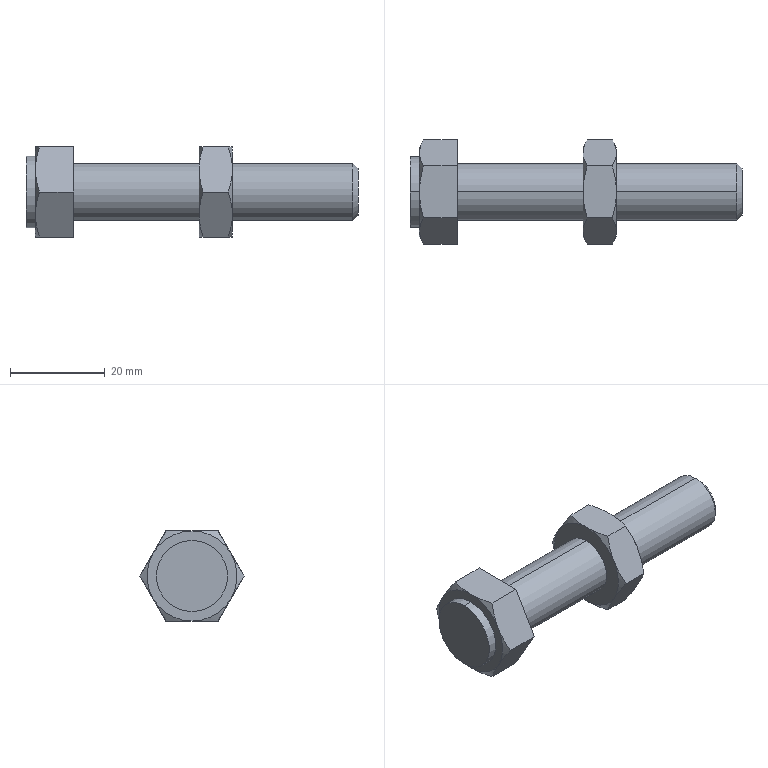Part | STEP file | 11-UST12-6011 | 2 solids | 48 faces | box 70 x 21.939 x 19 mm | volume 11194 mm3 | cone 24 | plane 18 | cylinder 6 | commonest cylinder face diameters 10.106 x2 12 x2 15 x2
STEP:
#1=CARTESIAN_POINT('',(58.926,0.,6.));
#2=VERTEX_POINT('',#1);
#3=CARTESIAN_POINT('',(58.926,0.,-6.));
#4=VERTEX_POINT('',#3);
#5=CARTESIAN_POINT('',(58.926,0.,0.));
#6=DIRECTION('',(-1.,0.,0.));
#7=DIRECTION('',(0.,0.,1.));
#8=AXIS2_PLACEMENT_3D('',#5,#6,#7);
#9=CIRCLE('',#8,6.);
#10=EDGE_CURVE('',#2,#4,#9,.T.);
#11=ORIENTED_EDGE('',*,*,#10,.T.);
#12=CARTESIAN_POINT('',(0.,0.,-6.));
#13=VERTEX_POINT('',#12);
#14=CARTESIAN_POINT('',(60.,0.,-6.));
#15=DIRECTION('',(-1.,0.,0.));
#16=VECTOR('',#15,1000.);
#17=LINE('',#14,#16);
#18=EDGE_CURVE('',#4,#13,#17,.T.);
#19=ORIENTED_EDGE('',*,*,#18,.T.);
#20=CARTESIAN_POINT('',(0.,0.,6.));
#21=VERTEX_POINT('',#20);
#22=CARTESIAN_POINT('',(0.,0.,0.));
#23=DIRECTION('',(-1.,0.,0.));
#24=DIRECTION('',(0.,0.,1.));
#25=AXIS2_PLACEMENT_3D('',#22,#23,#24);
#26=CIRCLE('',#25,6.);
#27=EDGE_CURVE('',#21,#13,#26,.T.);
#28=ORIENTED_EDGE('',*,*,#27,.F.);
#29=CARTESIAN_POINT('',(60.,0.,6.));
#30=DIRECTION('',(-1.,0.,0.));
#31=VECTOR('',#30,1000.);
#32=LINE('',#29,#31);
#33=EDGE_CURVE('',#2,#21,#32,.T.);
#34=ORIENTED_EDGE('',*,*,#33,.F.);
#35=EDGE_LOOP('',(#11,#19,#28,#34));
#36=FACE_OUTER_BOUND('',#35,.T.);
#37=CARTESIAN_POINT('',(60.,0.,0.));
#38=DIRECTION('',(-1.,0.,0.));
#39=DIRECTION('',(0.,0.,1.));
#40=AXIS2_PLACEMENT_3D('',#37,#38,#39);
#41=CYLINDRICAL_SURFACE('',#40,6.);
#42=ADVANCED_FACE('',(#36),#41,.T.);
#43=CARTESIAN_POINT('',(60.,0.,4.926));
#44=VERTEX_POINT('',#43);
#45=CARTESIAN_POINT('',(60.,0.,-4.926));
#46=VERTEX_POINT('',#45);
#47=CARTESIAN_POINT('',(60.,0.,0.));
#48=DIRECTION('',(-1.,0.,0.));
#49=DIRECTION('',(0.,0.,1.));
#50=AXIS2_PLACEMENT_3D('',#47,#48,#49);
#51=CIRCLE('',#50,4.926);
#52=EDGE_CURVE('',#44,#46,#51,.T.);
#53=ORIENTED_EDGE('',*,*,#52,.T.);
#54=CARTESIAN_POINT('',(60.,0.,-4.926));
#55=DIRECTION('',(-0.7071,0.,-0.7071));
#56=VECTOR('',#55,1000.);
#57=LINE('',#54,#56);
#58=EDGE_CURVE('',#46,#4,#57,.T.);
#59=ORIENTED_EDGE('',*,*,#58,.T.);
#60=ORIENTED_EDGE('',*,*,#10,.F.);
#61=CARTESIAN_POINT('',(60.,0.,4.926));
#62=DIRECTION('',(-0.7071,0.,0.7071));
#63=VECTOR('',#62,1000.);
#64=LINE('',#61,#63);
#65=EDGE_CURVE('',#44,#2,#64,.T.);
#66=ORIENTED_EDGE('',*,*,#65,.F.);
#67=EDGE_LOOP('',(#53,#59,#60,#66));
#68=FACE_OUTER_BOUND('',#67,.T.);
#69=CARTESIAN_POINT('',(60.,0.,0.));
#70=DIRECTION('',(-1.,0.,0.));
#71=DIRECTION('',(0.,0.,1.));
#72=AXIS2_PLACEMENT_3D('',#69,#70,#71);
#73=CONICAL_SURFACE('',#72,4.926,0.7854);
#74=ADVANCED_FACE('',(#68),#73,.T.);
#75=CARTESIAN_POINT('',(-8.,0.,7.5));
#76=VERTEX_POINT('',#75);
#77=CARTESIAN_POINT('',(-8.,0.,-7.5));
#78=VERTEX_POINT('',#77);
#79=CARTESIAN_POINT('',(-8.,0.,0.));
#80=DIRECTION('',(-1.,0.,0.));
#81=DIRECTION('',(0.,0.,1.));
#82=AXIS2_PLACEMENT_3D('',#79,#80,#81);
#83=CIRCLE('',#82,7.5);
#84=EDGE_CURVE('',#76,#78,#83,.T.);
#85=ORIENTED_EDGE('',*,*,#84,.T.);
#86=CARTESIAN_POINT('',(-10.,0.,-7.5));
#87=VERTEX_POINT('',#86);
#88=CARTESIAN_POINT('',(60.,0.,-7.5));
#89=DIRECTION('',(-1.,0.,0.));
#90=VECTOR('',#89,1000.);
#91=LINE('',#88,#90);
#92=EDGE_CURVE('',#78,#87,#91,.T.);
#93=ORIENTED_EDGE('',*,*,#92,.T.);
#94=CARTESIAN_POINT('',(-10.,0.,7.5));
#95=VERTEX_POINT('',#94);
#96=CARTESIAN_POINT('',(-10.,0.,0.));
#97=DIRECTION('',(-1.,0.,0.));
#98=DIRECTION('',(0.,0.,1.));
#99=AXIS2_PLACEMENT_3D('',#96,#97,#98);
#100=CIRCLE('',#99,7.5);
#101=EDGE_CURVE('',#95,#87,#100,.T.);
#102=ORIENTED_EDGE('',*,*,#101,.F.);
#103=CARTESIAN_POINT('',(60.,0.,7.5));
#104=DIRECTION('',(-1.,0.,0.));
#105=VECTOR('',#104,1000.);
#106=LINE('',#103,#105);
#107=EDGE_CURVE('',#76,#95,#106,.T.);
#108=ORIENTED_EDGE('',*,*,#107,.F.);
#109=EDGE_LOOP('',(#85,#93,#102,#108));
#110=FACE_OUTER_BOUND('',#109,.T.);
#111=CARTESIAN_POINT('',(60.,0.,0.));
#112=DIRECTION('',(-1.,0.,0.));
#113=DIRECTION('',(0.,0.,1.));
#114=AXIS2_PLACEMENT_3D('',#111,#112,#113);
#115=CYLINDRICAL_SURFACE('',#114,7.5);
#116=ADVANCED_FACE('',(#110),#115,.T.);
#117=CARTESIAN_POINT('',(-7.151,5.485,-9.5));
#118=VERTEX_POINT('',#117);
#119=CARTESIAN_POINT('',(-8.,8.227,-4.75));
#120=VERTEX_POINT('',#119);
#121=CARTESIAN_POINT('',(-7.151,5.485,-9.5));
#122=CARTESIAN_POINT('',(-7.411,5.933,-8.723));
#123=CARTESIAN_POINT('',(-7.624,6.385,-7.94));
#124=CARTESIAN_POINT('',(-7.919,7.299,-6.358));
#125=CARTESIAN_POINT('',(-8.,7.76,-5.559));
#126=CARTESIAN_POINT('',(-8.,8.227,-4.75));
#127=B_SPLINE_CURVE_WITH_KNOTS('',3,(#121,#122,#123,#124,#125,#126),.UNSPECIFIED.,.F.,.F.,(4,2,4),(0.000000238,0.002775,0.00555),.UNSPECIFIED.);
#128=EDGE_CURVE('',#118,#120,#127,.T.);
#129=ORIENTED_EDGE('',*,*,#128,.F.);
#130=CARTESIAN_POINT('',(-8.,0.,-9.5));
#131=VERTEX_POINT('',#130);
#132=CARTESIAN_POINT('',(-8.,0.,-9.5));
#133=CARTESIAN_POINT('',(-8.,0.9275,-9.5));
#134=CARTESIAN_POINT('',(-7.918,1.868,-9.5));
#135=CARTESIAN_POINT('',(-7.621,3.699,-9.5));
#136=CARTESIAN_POINT('',(-7.408,4.598,-9.5));
#137=CARTESIAN_POINT('',(-7.151,5.485,-9.5));
#138=B_SPLINE_CURVE_WITH_KNOTS('',3,(#132,#133,#134,#135,#136,#137),.UNSPECIFIED.,.F.,.F.,(4,2,4),(0.01537,0.01815,0.02093),.UNSPECIFIED.);
#139=EDGE_CURVE('',#131,#118,#138,.T.);
#140=ORIENTED_EDGE('',*,*,#139,.F.);
#141=CARTESIAN_POINT('',(-8.,0.,0.));
#142=DIRECTION('',(-1.,0.,0.));
#143=DIRECTION('',(0.,0.,1.));
#144=AXIS2_PLACEMENT_3D('',#141,#142,#143);
#145=CIRCLE('',#144,9.5);
#146=EDGE_CURVE('',#120,#131,#145,.T.);
#147=ORIENTED_EDGE('',*,*,#146,.F.);
#148=EDGE_LOOP('',(#129,#140,#147));
#149=FACE_OUTER_BOUND('',#148,.T.);
#150=CARTESIAN_POINT('',(-6.903,0.,0.));
#151=DIRECTION('',(1.,0.,0.));
#152=DIRECTION('',(0.,0.,-1.));
#153=AXIS2_PLACEMENT_3D('',#150,#151,#152);
#154=CONICAL_SURFACE('',#153,11.4,1.047);
#155=ADVANCED_FACE('',(#149),#154,.T.);
#156=CARTESIAN_POINT('',(-7.151,10.97,0.));
#157=VERTEX_POINT('',#156);
#158=CARTESIAN_POINT('',(-8.,8.227,-4.75));
#159=CARTESIAN_POINT('',(-8.,8.46,-4.347));
#160=CARTESIAN_POINT('',(-7.98,8.694,-3.942));
#161=CARTESIAN_POINT('',(-7.902,9.156,-3.141));
#162=CARTESIAN_POINT('',(-7.845,9.386,-2.743));
#163=CARTESIAN_POINT('',(-7.623,10.071,-1.557));
#164=CARTESIAN_POINT('',(-7.41,10.522,-0.7751));
#165=CARTESIAN_POINT('',(-7.151,10.97,0.));
#166=B_SPLINE_CURVE_WITH_KNOTS('',3,(#158,#159,#160,#161,#162,#163,#164,#165),.UNSPECIFIED.,.F.,.F.,(4,2,2,4),(0.00555,0.006932,0.008314,0.01108),.UNSPECIFIED.);
#167=EDGE_CURVE('',#120,#157,#166,.T.);
#168=ORIENTED_EDGE('',*,*,#167,.F.);
#169=CARTESIAN_POINT('',(-8.,8.227,4.75));
#170=VERTEX_POINT('',#169);
#171=CARTESIAN_POINT('',(-8.,0.,0.));
#172=DIRECTION('',(-1.,0.,0.));
#173=DIRECTION('',(0.,0.,1.));
#174=AXIS2_PLACEMENT_3D('',#171,#172,#173);
#175=CIRCLE('',#174,9.5);
#176=EDGE_CURVE('',#170,#120,#175,.T.);
#177=ORIENTED_EDGE('',*,*,#176,.F.);
#178=CARTESIAN_POINT('',(-7.151,10.97,0.));
#179=CARTESIAN_POINT('',(-7.411,10.521,0.777));
#180=CARTESIAN_POINT('',(-7.624,10.069,1.56));
#181=CARTESIAN_POINT('',(-7.919,9.156,3.142));
#182=CARTESIAN_POINT('',(-8.,8.694,3.941));
#183=CARTESIAN_POINT('',(-8.,8.227,4.75));
#184=B_SPLINE_CURVE_WITH_KNOTS('',3,(#178,#179,#180,#181,#182,#183),.UNSPECIFIED.,.F.,.F.,(4,2,4),(0.000000238,0.002775,0.00555),.UNSPECIFIED.);
#185=EDGE_CURVE('',#157,#170,#184,.T.);
#186=ORIENTED_EDGE('',*,*,#185,.F.);
#187=EDGE_LOOP('',(#168,#177,#186));
#188=FACE_OUTER_BOUND('',#187,.T.);
#189=CARTESIAN_POINT('',(-6.903,0.,0.));
#190=DIRECTION('',(1.,0.,0.));
#191=DIRECTION('',(0.,0.,-1.));
#192=AXIS2_PLACEMENT_3D('',#189,#190,#191);
#193=CONICAL_SURFACE('',#192,11.4,1.047);
#194=ADVANCED_FACE('',(#188),#193,.T.);
#195=CARTESIAN_POINT('',(-7.151,5.485,9.5));
#196=VERTEX_POINT('',#195);
#197=CARTESIAN_POINT('',(-8.,8.227,4.75));
#198=CARTESIAN_POINT('',(-8.,7.995,5.153));
#199=CARTESIAN_POINT('',(-7.98,7.761,5.558));
#200=CARTESIAN_POINT('',(-7.902,7.298,6.359));
#201=CARTESIAN_POINT('',(-7.845,7.069,6.757));
#202=CARTESIAN_POINT('',(-7.623,6.384,7.943));
#203=CARTESIAN_POINT('',(-7.41,5.932,8.725));
#204=CARTESIAN_POINT('',(-7.151,5.485,9.5));
#205=B_SPLINE_CURVE_WITH_KNOTS('',3,(#197,#198,#199,#200,#201,#202,#203,#204),.UNSPECIFIED.,.F.,.F.,(4,2,2,4),(0.00555,0.006932,0.008314,0.01108),.UNSPECIFIED.);
#206=EDGE_CURVE('',#170,#196,#205,.T.);
#207=ORIENTED_EDGE('',*,*,#206,.F.);
#208=CARTESIAN_POINT('',(-8.,0.,9.5));
#209=VERTEX_POINT('',#208);
#210=CARTESIAN_POINT('',(-8.,0.,0.));
#211=DIRECTION('',(-1.,0.,0.));
#212=DIRECTION('',(0.,0.,1.));
#213=AXIS2_PLACEMENT_3D('',#210,#211,#212);
#214=CIRCLE('',#213,9.5);
#215=EDGE_CURVE('',#209,#170,#214,.T.);
#216=ORIENTED_EDGE('',*,*,#215,.F.);
#217=CARTESIAN_POINT('',(-7.151,5.485,9.5));
#218=CARTESIAN_POINT('',(-7.408,4.598,9.5));
#219=CARTESIAN_POINT('',(-7.621,3.699,9.5));
#220=CARTESIAN_POINT('',(-7.918,1.868,9.5));
#221=CARTESIAN_POINT('',(-8.,0.9275,9.5));
#222=CARTESIAN_POINT('',(-8.,0.,9.5));
#223=B_SPLINE_CURVE_WITH_KNOTS('',3,(#217,#218,#219,#220,#221,#222),.UNSPECIFIED.,.F.,.F.,(4,2,4),(0.02408,0.02686,0.02964),.UNSPECIFIED.);
#224=EDGE_CURVE('',#196,#209,#223,.T.);
#225=ORIENTED_EDGE('',*,*,#224,.F.);
#226=EDGE_LOOP('',(#207,#216,#225));
#227=FACE_OUTER_BOUND('',#226,.T.);
#228=CARTESIAN_POINT('',(-6.903,0.,0.));
#229=DIRECTION('',(1.,0.,0.));
#230=DIRECTION('',(0.,0.,-1.));
#231=AXIS2_PLACEMENT_3D('',#228,#229,#230);
#232=CONICAL_SURFACE('',#231,11.4,1.047);
#233=ADVANCED_FACE('',(#227),#232,.T.);
#234=CARTESIAN_POINT('',(-7.151,-5.485,-9.5));
#235=VERTEX_POINT('',#234);
#236=CARTESIAN_POINT('',(-7.151,-5.485,-9.5));
#237=CARTESIAN_POINT('',(-7.409,-4.593,-9.5));
#238=CARTESIAN_POINT('',(-7.625,-3.679,-9.5));
#239=CARTESIAN_POINT('',(-7.92,-1.848,-9.5));
#240=CARTESIAN_POINT('',(-8.,-0.927,-9.5));
#241=CARTESIAN_POINT('',(-8.,0.,-9.5));
#242=B_SPLINE_CURVE_WITH_KNOTS('',3,(#236,#237,#238,#239,#240,#241),.UNSPECIFIED.,.F.,.F.,(4,2,4),(0.009824,0.0126,0.01537),.UNSPECIFIED.);
#243=EDGE_CURVE('',#235,#131,#242,.T.);
#244=ORIENTED_EDGE('',*,*,#243,.F.);
#245=CARTESIAN_POINT('',(-8.,-8.227,-4.75));
#246=VERTEX_POINT('',#245);
#247=CARTESIAN_POINT('',(-8.,-8.227,-4.75));
#248=CARTESIAN_POINT('',(-8.,-7.995,-5.153));
#249=CARTESIAN_POINT('',(-7.98,-7.761,-5.558));
#250=CARTESIAN_POINT('',(-7.902,-7.298,-6.359));
#251=CARTESIAN_POINT('',(-7.845,-7.069,-6.757));
#252=CARTESIAN_POINT('',(-7.623,-6.384,-7.943));
#253=CARTESIAN_POINT('',(-7.41,-5.932,-8.725));
#254=CARTESIAN_POINT('',(-7.151,-5.485,-9.5));
#255=B_SPLINE_CURVE_WITH_KNOTS('',3,(#247,#248,#249,#250,#251,#252,#253,#254),.UNSPECIFIED.,.F.,.F.,(4,2,2,4),(0.00555,0.006932,0.008314,0.01108),.UNSPECIFIED.);
#256=EDGE_CURVE('',#246,#235,#255,.T.);
#257=ORIENTED_EDGE('',*,*,#256,.F.);
#258=CARTESIAN_POINT('',(-8.,0.,0.));
#259=DIRECTION('',(-1.,0.,0.));
#260=DIRECTION('',(0.,0.,1.));
#261=AXIS2_PLACEMENT_3D('',#258,#259,#260);
#262=CIRCLE('',#261,9.5);
#263=EDGE_CURVE('',#131,#246,#262,.T.);
#264=ORIENTED_EDGE('',*,*,#263,.F.);
#265=EDGE_LOOP('',(#244,#257,#264));
#266=FACE_OUTER_BOUND('',#265,.T.);
#267=CARTESIAN_POINT('',(-6.903,0.,0.));
#268=DIRECTION('',(1.,0.,0.));
#269=DIRECTION('',(0.,0.,-1.));
#270=AXIS2_PLACEMENT_3D('',#267,#268,#269);
#271=CONICAL_SURFACE('',#270,11.4,1.047);
#272=ADVANCED_FACE('',(#266),#271,.T.);
#273=CARTESIAN_POINT('',(-7.151,-5.485,9.5));
#274=VERTEX_POINT('',#273);
#275=CARTESIAN_POINT('',(-8.,0.,9.5));
#276=CARTESIAN_POINT('',(-8.,-0.927,9.5));
#277=CARTESIAN_POINT('',(-7.92,-1.848,9.5));
#278=CARTESIAN_POINT('',(-7.625,-3.679,9.5));
#279=CARTESIAN_POINT('',(-7.409,-4.593,9.5));
#280=CARTESIAN_POINT('',(-7.151,-5.485,9.5));
#281=B_SPLINE_CURVE_WITH_KNOTS('',3,(#275,#276,#277,#278,#279,#280),.UNSPECIFIED.,.F.,.F.,(4,2,4),(0.02964,0.03241,0.03519),.UNSPECIFIED.);
#282=EDGE_CURVE('',#209,#274,#281,.T.);
#283=ORIENTED_EDGE('',*,*,#282,.F.);
#284=CARTESIAN_POINT('',(-8.,-8.227,4.75));
#285=VERTEX_POINT('',#284);
#286=CARTESIAN_POINT('',(-8.,0.,0.));
#287=DIRECTION('',(-1.,0.,0.));
#288=DIRECTION('',(0.,0.,1.));
#289=AXIS2_PLACEMENT_3D('',#286,#287,#288);
#290=CIRCLE('',#289,9.5);
#291=EDGE_CURVE('',#285,#209,#290,.T.);
#292=ORIENTED_EDGE('',*,*,#291,.F.);
#293=CARTESIAN_POINT('',(-7.151,-5.485,9.5));
#294=CARTESIAN_POINT('',(-7.411,-5.933,8.723));
#295=CARTESIAN_POINT('',(-7.624,-6.385,7.94));
#296=CARTESIAN_POINT('',(-7.919,-7.299,6.358));
#297=CARTESIAN_POINT('',(-8.,-7.76,5.559));
#298=CARTESIAN_POINT('',(-8.,-8.227,4.75));
#299=B_SPLINE_CURVE_WITH_KNOTS('',3,(#293,#294,#295,#296,#297,#298),.UNSPECIFIED.,.F.,.F.,(4,2,4),(0.000000238,0.002775,0.00555),.UNSPECIFIED.);
#300=EDGE_CURVE('',#274,#285,#299,.T.);
#301=ORIENTED_EDGE('',*,*,#300,.F.);
#302=EDGE_LOOP('',(#283,#292,#301));
#303=FACE_OUTER_BOUND('',#302,.T.);
#304=CARTESIAN_POINT('',(-6.903,0.,0.));
#305=DIRECTION('',(1.,0.,0.));
#306=DIRECTION('',(0.,0.,-1.));
#307=AXIS2_PLACEMENT_3D('',#304,#305,#306);
#308=CONICAL_SURFACE('',#307,11.4,1.047);
#309=ADVANCED_FACE('',(#303),#308,.T.);
#310=CARTESIAN_POINT('',(-7.151,-10.97,0.));
#311=VERTEX_POINT('',#310);
#312=CARTESIAN_POINT('',(-7.151,-10.97,0.));
#313=CARTESIAN_POINT('',(-7.411,-10.521,-0.777));
#314=CARTESIAN_POINT('',(-7.624,-10.069,-1.56));
#315=CARTESIAN_POINT('',(-7.919,-9.156,-3.142));
#316=CARTESIAN_POINT('',(-8.,-8.694,-3.941));
#317=CARTESIAN_POINT('',(-8.,-8.227,-4.75));
#318=B_SPLINE_CURVE_WITH_KNOTS('',3,(#312,#313,#314,#315,#316,#317),.UNSPECIFIED.,.F.,.F.,(4,2,4),(0.000000238,0.002775,0.00555),.UNSPECIFIED.);
#319=EDGE_CURVE('',#311,#246,#318,.T.);
#320=ORIENTED_EDGE('',*,*,#319,.F.);
#321=CARTESIAN_POINT('',(-8.,-8.227,4.75));
#322=CARTESIAN_POINT('',(-8.,-8.46,4.347));
#323=CARTESIAN_POINT('',(-7.98,-8.694,3.942));
#324=CARTESIAN_POINT('',(-7.902,-9.156,3.141));
#325=CARTESIAN_POINT('',(-7.845,-9.386,2.743));
#326=CARTESIAN_POINT('',(-7.623,-10.071,1.557));
#327=CARTESIAN_POINT('',(-7.41,-10.522,0.7751));
#328=CARTESIAN_POINT('',(-7.151,-10.97,0.));
#329=B_SPLINE_CURVE_WITH_KNOTS('',3,(#321,#322,#323,#324,#325,#326,#327,#328),.UNSPECIFIED.,.F.,.F.,(4,2,2,4),(0.00555,0.006932,0.008314,0.01108),.UNSPECIFIED.);
#330=EDGE_CURVE('',#285,#311,#329,.T.);
#331=ORIENTED_EDGE('',*,*,#330,.F.);
#332=CARTESIAN_POINT('',(-8.,0.,0.));
#333=DIRECTION('',(-1.,0.,0.));
#334=DIRECTION('',(0.,0.,1.));
#335=AXIS2_PLACEMENT_3D('',#332,#333,#334);
#336=CIRCLE('',#335,9.5);
#337=EDGE_CURVE('',#246,#285,#336,.T.);
#338=ORIENTED_EDGE('',*,*,#337,.F.);
#339=EDGE_LOOP('',(#320,#331,#338));
#340=FACE_OUTER_BOUND('',#339,.T.);
#341=CARTESIAN_POINT('',(-6.903,0.,0.));
#342=DIRECTION('',(1.,0.,0.));
#343=DIRECTION('',(0.,0.,-1.));
#344=AXIS2_PLACEMENT_3D('',#341,#342,#343);
#345=CONICAL_SURFACE('',#344,11.4,1.047);
#346=ADVANCED_FACE('',(#340),#345,.T.);
#347=ORIENTED_EDGE('',*,*,#101,.T.);
#348=CARTESIAN_POINT('',(-10.,0.,0.));
#349=DIRECTION('',(-1.,0.,0.));
#350=DIRECTION('',(0.,0.,1.));
#351=AXIS2_PLACEMENT_3D('',#348,#349,#350);
#352=CIRCLE('',#351,7.5);
#353=EDGE_CURVE('',#87,#95,#352,.T.);
#354=ORIENTED_EDGE('',*,*,#353,.T.);
#355=EDGE_LOOP('',(#347,#354));
#356=FACE_OUTER_BOUND('',#355,.T.);
#357=CARTESIAN_POINT('',(-10.,0.,0.));
#358=DIRECTION('',(1.,0.,0.));
#359=DIRECTION('',(0.,0.,-1.));
#360=AXIS2_PLACEMENT_3D('',#357,#358,#359);
#361=PLANE('',#360);
#362=ADVANCED_FACE('',(#356),#361,.F.);
#363=ORIENTED_EDGE('',*,*,#92,.F.);
#364=CARTESIAN_POINT('',(-8.,0.,0.));
#365=DIRECTION('',(-1.,0.,0.));
#366=DIRECTION('',(0.,0.,1.));
#367=AXIS2_PLACEMENT_3D('',#364,#365,#366);
#368=CIRCLE('',#367,7.5);
#369=EDGE_CURVE('',#78,#76,#368,.T.);
#370=ORIENTED_EDGE('',*,*,#369,.T.);
#371=ORIENTED_EDGE('',*,*,#107,.T.);
#372=ORIENTED_EDGE('',*,*,#353,.F.);
#373=EDGE_LOOP('',(#363,#370,#371,#372));
#374=FACE_OUTER_BOUND('',#373,.T.);
#375=CARTESIAN_POINT('',(60.,0.,0.));
#376=DIRECTION('',(-1.,0.,0.));
#377=DIRECTION('',(0.,0.,1.));
#378=AXIS2_PLACEMENT_3D('',#375,#376,#377);
#379=CYLINDRICAL_SURFACE('',#378,7.5);
#380=ADVANCED_FACE('',(#374),#379,.T.);
#381=ORIENTED_EDGE('',*,*,#84,.F.);
#382=ORIENTED_EDGE('',*,*,#369,.F.);
#383=EDGE_LOOP('',(#381,#382));
#384=FACE_BOUND('',#383,.T.);
#385=ORIENTED_EDGE('',*,*,#215,.T.);
#386=ORIENTED_EDGE('',*,*,#176,.T.);
#387=ORIENTED_EDGE('',*,*,#146,.T.);
#388=ORIENTED_EDGE('',*,*,#263,.T.);
#389=ORIENTED_EDGE('',*,*,#337,.T.);
#390=ORIENTED_EDGE('',*,*,#291,.T.);
#391=EDGE_LOOP('',(#385,#386,#387,#388,#389,#390));
#392=FACE_OUTER_BOUND('',#391,.T.);
#393=CARTESIAN_POINT('',(-8.,7.5,0.));
#394=DIRECTION('',(1.,0.,0.));
#395=DIRECTION('',(0.,0.,-1.));
#396=AXIS2_PLACEMENT_3D('',#393,#394,#395);
#397=PLANE('',#396);
#398=ADVANCED_FACE('',(#384,#392),#397,.F.);
#399=ORIENTED_EDGE('',*,*,#224,.T.);
#400=ORIENTED_EDGE('',*,*,#282,.T.);
#401=CARTESIAN_POINT('',(0.,-5.485,9.5));
#402=VERTEX_POINT('',#401);
#403=CARTESIAN_POINT('',(-10.,-5.485,9.5));
#404=DIRECTION('',(1.,0.,0.));
#405=VECTOR('',#404,1000.);
#406=LINE('',#403,#405);
#407=EDGE_CURVE('',#274,#402,#406,.T.);
#408=ORIENTED_EDGE('',*,*,#407,.T.);
#409=CARTESIAN_POINT('',(0.,5.485,9.5));
#410=VERTEX_POINT('',#409);
#411=CARTESIAN_POINT('',(0.,5.485,9.5));
#412=DIRECTION('',(0.,-1.,0.));
#413=VECTOR('',#412,1000.);
#414=LINE('',#411,#413);
#415=EDGE_CURVE('',#410,#402,#414,.T.);
#416=ORIENTED_EDGE('',*,*,#415,.F.);
#417=CARTESIAN_POINT('',(-10.,5.485,9.5));
#418=DIRECTION('',(1.,0.,0.));
#419=VECTOR('',#418,1000.);
#420=LINE('',#417,#419);
#421=EDGE_CURVE('',#196,#410,#420,.T.);
#422=ORIENTED_EDGE('',*,*,#421,.F.);
#423=EDGE_LOOP('',(#399,#400,#408,#416,#422));
#424=FACE_OUTER_BOUND('',#423,.T.);
#425=CARTESIAN_POINT('',(-10.,5.485,9.5));
#426=DIRECTION('',(0.,0.,1.));
#427=DIRECTION('',(1.,0.,0.));
#428=AXIS2_PLACEMENT_3D('',#425,#426,#427);
#429=PLANE('',#428);
#430=ADVANCED_FACE('',(#424),#429,.T.);
#431=ORIENTED_EDGE('',*,*,#185,.T.);
#432=ORIENTED_EDGE('',*,*,#206,.T.);
#433=ORIENTED_EDGE('',*,*,#421,.T.);
#434=CARTESIAN_POINT('',(0.,10.97,0.));
#435=VERTEX_POINT('',#434);
#436=CARTESIAN_POINT('',(0.,10.97,0.));
#437=DIRECTION('',(0.,-0.5,0.866));
#438=VECTOR('',#437,1000.);
#439=LINE('',#436,#438);
#440=EDGE_CURVE('',#435,#410,#439,.T.);
#441=ORIENTED_EDGE('',*,*,#440,.F.);
#442=CARTESIAN_POINT('',(-10.,10.97,0.));
#443=DIRECTION('',(1.,0.,0.));
#444=VECTOR('',#443,1000.);
#445=LINE('',#442,#444);
#446=EDGE_CURVE('',#157,#435,#445,.T.);
#447=ORIENTED_EDGE('',*,*,#446,.F.);
#448=EDGE_LOOP('',(#431,#432,#433,#441,#447));
#449=FACE_OUTER_BOUND('',#448,.T.);
#450=CARTESIAN_POINT('',(-10.,10.97,0.));
#451=DIRECTION('',(0.,0.866,0.5));
#452=DIRECTION('',(0.,-0.5,0.866));
#453=AXIS2_PLACEMENT_3D('',#450,#451,#452);
#454=PLANE('',#453);
#455=ADVANCED_FACE('',(#449),#454,.T.);
#456=ORIENTED_EDGE('',*,*,#128,.T.);
#457=ORIENTED_EDGE('',*,*,#167,.T.);
#458=ORIENTED_EDGE('',*,*,#446,.T.);
#459=CARTESIAN_POINT('',(0.,5.485,-9.5));
#460=VERTEX_POINT('',#459);
#461=CARTESIAN_POINT('',(0.,5.485,-9.5));
#462=DIRECTION('',(0.,0.5,0.866));
#463=VECTOR('',#462,1000.);
#464=LINE('',#461,#463);
#465=EDGE_CURVE('',#460,#435,#464,.T.);
#466=ORIENTED_EDGE('',*,*,#465,.F.);
#467=CARTESIAN_POINT('',(-10.,5.485,-9.5));
#468=DIRECTION('',(1.,0.,0.));
#469=VECTOR('',#468,1000.);
#470=LINE('',#467,#469);
#471=EDGE_CURVE('',#118,#460,#470,.T.);
#472=ORIENTED_EDGE('',*,*,#471,.F.);
#473=EDGE_LOOP('',(#456,#457,#458,#466,#472));
#474=FACE_OUTER_BOUND('',#473,.T.);
#475=CARTESIAN_POINT('',(-10.,5.485,-9.5));
#476=DIRECTION('',(0.,0.866,-0.5));
#477=DIRECTION('',(0.,0.5,0.866));
#478=AXIS2_PLACEMENT_3D('',#475,#476,#477);
#479=PLANE('',#478);
#480=ADVANCED_FACE('',(#474),#479,.T.);
#481=ORIENTED_EDGE('',*,*,#243,.T.);
#482=ORIENTED_EDGE('',*,*,#139,.T.);
#483=ORIENTED_EDGE('',*,*,#471,.T.);
#484=CARTESIAN_POINT('',(0.,-5.485,-9.5));
#485=VERTEX_POINT('',#484);
#486=CARTESIAN_POINT('',(0.,-5.485,-9.5));
#487=DIRECTION('',(0.,1.,0.));
#488=VECTOR('',#487,1000.);
#489=LINE('',#486,#488);
#490=EDGE_CURVE('',#485,#460,#489,.T.);
#491=ORIENTED_EDGE('',*,*,#490,.F.);
#492=CARTESIAN_POINT('',(-10.,-5.485,-9.5));
#493=DIRECTION('',(1.,0.,0.));
#494=VECTOR('',#493,1000.);
#495=LINE('',#492,#494);
#496=EDGE_CURVE('',#235,#485,#495,.T.);
#497=ORIENTED_EDGE('',*,*,#496,.F.);
#498=EDGE_LOOP('',(#481,#482,#483,#491,#497));
#499=FACE_OUTER_BOUND('',#498,.T.);
#500=CARTESIAN_POINT('',(-10.,-5.485,-9.5));
#501=DIRECTION('',(0.,0.,-1.));
#502=DIRECTION('',(-1.,0.,0.));
#503=AXIS2_PLACEMENT_3D('',#500,#501,#502);
#504=PLANE('',#503);
#505=ADVANCED_FACE('',(#499),#504,.T.);
#506=ORIENTED_EDGE('',*,*,#319,.T.);
#507=ORIENTED_EDGE('',*,*,#256,.T.);
#508=ORIENTED_EDGE('',*,*,#496,.T.);
#509=CARTESIAN_POINT('',(0.,-10.97,0.));
#510=VERTEX_POINT('',#509);
#511=CARTESIAN_POINT('',(0.,-10.97,0.));
#512=DIRECTION('',(0.,0.5,-0.866));
#513=VECTOR('',#512,1000.);
#514=LINE('',#511,#513);
#515=EDGE_CURVE('',#510,#485,#514,.T.);
#516=ORIENTED_EDGE('',*,*,#515,.F.);
#517=CARTESIAN_POINT('',(-10.,-10.97,0.));
#518=DIRECTION('',(1.,0.,0.));
#519=VECTOR('',#518,1000.);
#520=LINE('',#517,#519);
#521=EDGE_CURVE('',#311,#510,#520,.T.);
#522=ORIENTED_EDGE('',*,*,#521,.F.);
#523=EDGE_LOOP('',(#506,#507,#508,#516,#522));
#524=FACE_OUTER_BOUND('',#523,.T.);
#525=CARTESIAN_POINT('',(-10.,-10.97,0.));
#526=DIRECTION('',(0.,-0.866,-0.5));
#527=DIRECTION('',(0.,0.5,-0.866));
#528=AXIS2_PLACEMENT_3D('',#525,#526,#527);
#529=PLANE('',#528);
#530=ADVANCED_FACE('',(#524),#529,.T.);
#531=ORIENTED_EDGE('',*,*,#300,.T.);
#532=ORIENTED_EDGE('',*,*,#330,.T.);
#533=ORIENTED_EDGE('',*,*,#521,.T.);
#534=CARTESIAN_POINT('',(0.,-5.485,9.5));
#535=DIRECTION('',(0.,-0.5,-0.866));
#536=VECTOR('',#535,1000.);
#537=LINE('',#534,#536);
#538=EDGE_CURVE('',#402,#510,#537,.T.);
#539=ORIENTED_EDGE('',*,*,#538,.F.);
#540=ORIENTED_EDGE('',*,*,#407,.F.);
#541=EDGE_LOOP('',(#531,#532,#533,#539,#540));
#542=FACE_OUTER_BOUND('',#541,.T.);
#543=CARTESIAN_POINT('',(-10.,-5.485,9.5));
#544=DIRECTION('',(0.,-0.866,0.5));
#545=DIRECTION('',(0.,-0.5,-0.866));
#546=AXIS2_PLACEMENT_3D('',#543,#544,#545);
#547=PLANE('',#546);
#548=ADVANCED_FACE('',(#542),#547,.T.);
#549=ORIENTED_EDGE('',*,*,#52,.F.);
#550=CARTESIAN_POINT('',(60.,0.,0.));
#551=DIRECTION('',(-1.,0.,0.));
#552=DIRECTION('',(0.,0.,1.));
#553=AXIS2_PLACEMENT_3D('',#550,#551,#552);
#554=CIRCLE('',#553,4.926);
#555=EDGE_CURVE('',#46,#44,#554,.T.);
#556=ORIENTED_EDGE('',*,*,#555,.F.);
#557=EDGE_LOOP('',(#549,#556));
#558=FACE_OUTER_BOUND('',#557,.T.);
#559=CARTESIAN_POINT('',(60.,4.926,0.));
#560=DIRECTION('',(-1.,0.,0.));
#561=DIRECTION('',(0.,0.,1.));
#562=AXIS2_PLACEMENT_3D('',#559,#560,#561);
#563=PLANE('',#562);
#564=ADVANCED_FACE('',(#558),#563,.F.);
#565=ORIENTED_EDGE('',*,*,#58,.F.);
#566=ORIENTED_EDGE('',*,*,#555,.T.);
#567=ORIENTED_EDGE('',*,*,#65,.T.);
#568=CARTESIAN_POINT('',(58.926,0.,0.));
#569=DIRECTION('',(-1.,0.,0.));
#570=DIRECTION('',(0.,0.,1.));
#571=AXIS2_PLACEMENT_3D('',#568,#569,#570);
#572=CIRCLE('',#571,6.);
#573=EDGE_CURVE('',#4,#2,#572,.T.);
#574=ORIENTED_EDGE('',*,*,#573,.F.);
#575=EDGE_LOOP('',(#565,#566,#567,#574));
#576=FACE_OUTER_BOUND('',#575,.T.);
#577=CARTESIAN_POINT('',(60.,0.,0.));
#578=DIRECTION('',(-1.,0.,0.));
#579=DIRECTION('',(0.,0.,1.));
#580=AXIS2_PLACEMENT_3D('',#577,#578,#579);
#581=CONICAL_SURFACE('',#580,4.926,0.7854);
#582=ADVANCED_FACE('',(#576),#581,.T.);
#583=ORIENTED_EDGE('',*,*,#18,.F.);
#584=ORIENTED_EDGE('',*,*,#573,.T.);
#585=ORIENTED_EDGE('',*,*,#33,.T.);
#586=CARTESIAN_POINT('',(0.,0.,0.));
#587=DIRECTION('',(-1.,0.,0.));
#588=DIRECTION('',(0.,0.,1.));
#589=AXIS2_PLACEMENT_3D('',#586,#587,#588);
#590=CIRCLE('',#589,6.);
#591=EDGE_CURVE('',#13,#21,#590,.T.);
#592=ORIENTED_EDGE('',*,*,#591,.F.);
#593=EDGE_LOOP('',(#583,#584,#585,#592));
#594=FACE_OUTER_BOUND('',#593,.T.);
#595=CARTESIAN_POINT('',(60.,0.,0.));
#596=DIRECTION('',(-1.,0.,0.));
#597=DIRECTION('',(0.,0.,1.));
#598=AXIS2_PLACEMENT_3D('',#595,#596,#597);
#599=CYLINDRICAL_SURFACE('',#598,6.);
#600=ADVANCED_FACE('',(#594),#599,.T.);
#601=ORIENTED_EDGE('',*,*,#27,.T.);
#602=ORIENTED_EDGE('',*,*,#591,.T.);
#603=EDGE_LOOP('',(#601,#602));
#604=FACE_BOUND('',#603,.T.);
#605=ORIENTED_EDGE('',*,*,#415,.T.);
#606=ORIENTED_EDGE('',*,*,#538,.T.);
#607=ORIENTED_EDGE('',*,*,#515,.T.);
#608=ORIENTED_EDGE('',*,*,#490,.T.);
#609=ORIENTED_EDGE('',*,*,#465,.T.);
#610=ORIENTED_EDGE('',*,*,#440,.T.);
#611=EDGE_LOOP('',(#605,#606,#607,#608,#609,#610));
#612=FACE_OUTER_BOUND('',#611,.T.);
#613=CARTESIAN_POINT('',(0.,11.4,0.));
#614=DIRECTION('',(-1.,0.,0.));
#615=DIRECTION('',(0.,0.,1.));
#616=AXIS2_PLACEMENT_3D('',#613,#614,#615);
#617=PLANE('',#616);
#618=ADVANCED_FACE('',(#604,#612),#617,.F.);
#619=CLOSED_SHELL('',(#42,#74,#116,#155,#194,#233,#272,#309,#346,#362,#380,#398,#430,#455,#480,#505,#530,#548,#564,#582,#600,#618));
#620=MANIFOLD_SOLID_BREP('',#619);
#621=CARTESIAN_POINT('',(27.447,0.,-5.053));
#622=VERTEX_POINT('',#621);
#623=CARTESIAN_POINT('',(27.447,0.,5.053));
#624=VERTEX_POINT('',#623);
#625=CARTESIAN_POINT('',(27.447,0.,0.));
#626=DIRECTION('',(1.,0.,0.));
#627=DIRECTION('',(0.,0.,1.));
#628=AXIS2_PLACEMENT_3D('',#625,#626,#627);
#629=CIRCLE('',#628,5.053);
#630=EDGE_CURVE('',#622,#624,#629,.T.);
#631=ORIENTED_EDGE('',*,*,#630,.T.);
#632=CARTESIAN_POINT('',(26.5,0.,6.));
#633=VERTEX_POINT('',#632);
#634=CARTESIAN_POINT('',(26.5,0.,6.));
#635=DIRECTION('',(-0.7071,0.,0.7071));
#636=VECTOR('',#635,1000.);
#637=LINE('',#634,#636);
#638=EDGE_CURVE('',#624,#633,#637,.T.);
#639=ORIENTED_EDGE('',*,*,#638,.T.);
#640=CARTESIAN_POINT('',(26.5,0.,-6.));
#641=VERTEX_POINT('',#640);
#642=CARTESIAN_POINT('',(26.5,0.,0.));
#643=DIRECTION('',(1.,0.,0.));
#644=DIRECTION('',(0.,0.,1.));
#645=AXIS2_PLACEMENT_3D('',#642,#643,#644);
#646=CIRCLE('',#645,6.);
#647=EDGE_CURVE('',#641,#633,#646,.T.);
#648=ORIENTED_EDGE('',*,*,#647,.F.);
#649=CARTESIAN_POINT('',(26.5,0.,-6.));
#650=DIRECTION('',(-0.7071,0.,-0.7071));
#651=VECTOR('',#650,1000.);
#652=LINE('',#649,#651);
#653=EDGE_CURVE('',#622,#641,#652,.T.);
#654=ORIENTED_EDGE('',*,*,#653,.F.);
#655=EDGE_LOOP('',(#631,#639,#648,#654));
#656=FACE_OUTER_BOUND('',#655,.T.);
#657=CARTESIAN_POINT('',(26.5,0.,0.));
#658=DIRECTION('',(-1.,0.,0.));
#659=DIRECTION('',(0.,0.,-1.));
#660=AXIS2_PLACEMENT_3D('',#657,#658,#659);
#661=CONICAL_SURFACE('',#660,6.,0.7854);
#662=ADVANCED_FACE('',(#656),#661,.F.);
#663=ORIENTED_EDGE('',*,*,#630,.F.);
#664=CARTESIAN_POINT('',(32.553,0.,-5.053));
#665=VERTEX_POINT('',#664);
#666=CARTESIAN_POINT('',(26.5,0.,-5.053));
#667=DIRECTION('',(1.,0.,0.));
#668=VECTOR('',#667,1000.);
#669=LINE('',#666,#668);
#670=EDGE_CURVE('',#622,#665,#669,.T.);
#671=ORIENTED_EDGE('',*,*,#670,.T.);
#672=CARTESIAN_POINT('',(32.553,0.,5.053));
#673=VERTEX_POINT('',#672);
#674=CARTESIAN_POINT('',(32.553,0.,0.));
#675=DIRECTION('',(1.,0.,0.));
#676=DIRECTION('',(0.,0.,1.));
#677=AXIS2_PLACEMENT_3D('',#674,#675,#676);
#678=CIRCLE('',#677,5.053);
#679=EDGE_CURVE('',#665,#673,#678,.T.);
#680=ORIENTED_EDGE('',*,*,#679,.T.);
#681=CARTESIAN_POINT('',(26.5,0.,5.053));
#682=DIRECTION('',(1.,0.,0.));
#683=VECTOR('',#682,1000.);
#684=LINE('',#681,#683);
#685=EDGE_CURVE('',#624,#673,#684,.T.);
#686=ORIENTED_EDGE('',*,*,#685,.F.);
#687=EDGE_LOOP('',(#663,#671,#680,#686));
#688=FACE_OUTER_BOUND('',#687,.T.);
#689=CARTESIAN_POINT('',(26.5,0.,0.));
#690=DIRECTION('',(1.,0.,0.));
#691=DIRECTION('',(0.,0.,1.));
#692=AXIS2_PLACEMENT_3D('',#689,#690,#691);
#693=CYLINDRICAL_SURFACE('',#692,5.053);
#694=ADVANCED_FACE('',(#688),#693,.F.);
#695=ORIENTED_EDGE('',*,*,#679,.F.);
#696=CARTESIAN_POINT('',(33.5,0.,-6.));
#697=VERTEX_POINT('',#696);
#698=CARTESIAN_POINT('',(32.553,0.,-5.053));
#699=DIRECTION('',(0.7071,0.,-0.7071));
#700=VECTOR('',#699,1000.);
#701=LINE('',#698,#700);
#702=EDGE_CURVE('',#665,#697,#701,.T.);
#703=ORIENTED_EDGE('',*,*,#702,.T.);
#704=CARTESIAN_POINT('',(33.5,0.,6.));
#705=VERTEX_POINT('',#704);
#706=CARTESIAN_POINT('',(33.5,0.,0.));
#707=DIRECTION('',(1.,0.,0.));
#708=DIRECTION('',(0.,0.,1.));
#709=AXIS2_PLACEMENT_3D('',#706,#707,#708);
#710=CIRCLE('',#709,6.);
#711=EDGE_CURVE('',#697,#705,#710,.T.);
#712=ORIENTED_EDGE('',*,*,#711,.T.);
#713=CARTESIAN_POINT('',(32.553,0.,5.053));
#714=DIRECTION('',(0.7071,0.,0.7071));
#715=VECTOR('',#714,1000.);
#716=LINE('',#713,#715);
#717=EDGE_CURVE('',#673,#705,#716,.T.);
#718=ORIENTED_EDGE('',*,*,#717,.F.);
#719=EDGE_LOOP('',(#695,#703,#712,#718));
#720=FACE_OUTER_BOUND('',#719,.T.);
#721=CARTESIAN_POINT('',(32.553,0.,0.));
#722=DIRECTION('',(1.,0.,0.));
#723=DIRECTION('',(0.,0.,1.));
#724=AXIS2_PLACEMENT_3D('',#721,#722,#723);
#725=CONICAL_SURFACE('',#724,5.053,0.7854);
#726=ADVANCED_FACE('',(#720),#725,.F.);
#727=CARTESIAN_POINT('',(32.651,-5.485,-9.5));
#728=VERTEX_POINT('',#727);
#729=CARTESIAN_POINT('',(33.5,-8.227,-4.75));
#730=VERTEX_POINT('',#729);
#731=CARTESIAN_POINT('',(32.651,-5.485,-9.5));
#732=CARTESIAN_POINT('',(32.911,-5.933,-8.723));
#733=CARTESIAN_POINT('',(33.124,-6.385,-7.94));
#734=CARTESIAN_POINT('',(33.419,-7.299,-6.358));
#735=CARTESIAN_POINT('',(33.5,-7.76,-5.559));
#736=CARTESIAN_POINT('',(33.5,-8.227,-4.75));
#737=B_SPLINE_CURVE_WITH_KNOTS('',3,(#731,#732,#733,#734,#735,#736),.UNSPECIFIED.,.F.,.F.,(4,2,4),(0.000000238,0.002775,0.00555),.UNSPECIFIED.);
#738=EDGE_CURVE('',#728,#730,#737,.T.);
#739=ORIENTED_EDGE('',*,*,#738,.F.);
#740=CARTESIAN_POINT('',(33.5,0.,-9.5));
#741=VERTEX_POINT('',#740);
#742=CARTESIAN_POINT('',(33.5,0.,-9.5));
#743=CARTESIAN_POINT('',(33.5,-0.9275,-9.5));
#744=CARTESIAN_POINT('',(33.418,-1.868,-9.5));
#745=CARTESIAN_POINT('',(33.121,-3.699,-9.5));
#746=CARTESIAN_POINT('',(32.908,-4.598,-9.5));
#747=CARTESIAN_POINT('',(32.651,-5.485,-9.5));
#748=B_SPLINE_CURVE_WITH_KNOTS('',3,(#742,#743,#744,#745,#746,#747),.UNSPECIFIED.,.F.,.F.,(4,2,4),(0.01537,0.01815,0.02093),.UNSPECIFIED.);
#749=EDGE_CURVE('',#741,#728,#748,.T.);
#750=ORIENTED_EDGE('',*,*,#749,.F.);
#751=CARTESIAN_POINT('',(33.5,0.,0.));
#752=DIRECTION('',(1.,0.,0.));
#753=DIRECTION('',(0.,0.,1.));
#754=AXIS2_PLACEMENT_3D('',#751,#752,#753);
#755=CIRCLE('',#754,9.5);
#756=EDGE_CURVE('',#730,#741,#755,.T.);
#757=ORIENTED_EDGE('',*,*,#756,.F.);
#758=EDGE_LOOP('',(#739,#750,#757));
#759=FACE_OUTER_BOUND('',#758,.T.);
#760=CARTESIAN_POINT('',(32.403,0.,0.));
#761=DIRECTION('',(-1.,0.,0.));
#762=DIRECTION('',(0.,0.,-1.));
#763=AXIS2_PLACEMENT_3D('',#760,#761,#762);
#764=CONICAL_SURFACE('',#763,11.4,1.047);
#765=ADVANCED_FACE('',(#759),#764,.T.);
#766=CARTESIAN_POINT('',(32.651,-10.97,0.));
#767=VERTEX_POINT('',#766);
#768=CARTESIAN_POINT('',(33.5,-8.227,-4.75));
#769=CARTESIAN_POINT('',(33.5,-8.46,-4.347));
#770=CARTESIAN_POINT('',(33.48,-8.694,-3.942));
#771=CARTESIAN_POINT('',(33.402,-9.156,-3.141));
#772=CARTESIAN_POINT('',(33.345,-9.386,-2.743));
#773=CARTESIAN_POINT('',(33.123,-10.071,-1.557));
#774=CARTESIAN_POINT('',(32.91,-10.522,-0.7751));
#775=CARTESIAN_POINT('',(32.651,-10.97,0.));
#776=B_SPLINE_CURVE_WITH_KNOTS('',3,(#768,#769,#770,#771,#772,#773,#774,#775),.UNSPECIFIED.,.F.,.F.,(4,2,2,4),(0.00555,0.006932,0.008314,0.01108),.UNSPECIFIED.);
#777=EDGE_CURVE('',#730,#767,#776,.T.);
#778=ORIENTED_EDGE('',*,*,#777,.F.);
#779=CARTESIAN_POINT('',(33.5,-8.227,4.75));
#780=VERTEX_POINT('',#779);
#781=CARTESIAN_POINT('',(33.5,0.,0.));
#782=DIRECTION('',(1.,0.,0.));
#783=DIRECTION('',(0.,0.,1.));
#784=AXIS2_PLACEMENT_3D('',#781,#782,#783);
#785=CIRCLE('',#784,9.5);
#786=EDGE_CURVE('',#780,#730,#785,.T.);
#787=ORIENTED_EDGE('',*,*,#786,.F.);
#788=CARTESIAN_POINT('',(32.651,-10.97,0.));
#789=CARTESIAN_POINT('',(32.911,-10.521,0.777));
#790=CARTESIAN_POINT('',(33.124,-10.069,1.56));
#791=CARTESIAN_POINT('',(33.419,-9.156,3.142));
#792=CARTESIAN_POINT('',(33.5,-8.694,3.941));
#793=CARTESIAN_POINT('',(33.5,-8.227,4.75));
#794=B_SPLINE_CURVE_WITH_KNOTS('',3,(#788,#789,#790,#791,#792,#793),.UNSPECIFIED.,.F.,.F.,(4,2,4),(0.000000238,0.002775,0.00555),.UNSPECIFIED.);
#795=EDGE_CURVE('',#767,#780,#794,.T.);
#796=ORIENTED_EDGE('',*,*,#795,.F.);
#797=EDGE_LOOP('',(#778,#787,#796));
#798=FACE_OUTER_BOUND('',#797,.T.);
#799=CARTESIAN_POINT('',(32.403,0.,0.));
#800=DIRECTION('',(-1.,0.,0.));
#801=DIRECTION('',(0.,0.,-1.));
#802=AXIS2_PLACEMENT_3D('',#799,#800,#801);
#803=CONICAL_SURFACE('',#802,11.4,1.047);
#804=ADVANCED_FACE('',(#798),#803,.T.);
#805=CARTESIAN_POINT('',(32.651,-5.485,9.5));
#806=VERTEX_POINT('',#805);
#807=CARTESIAN_POINT('',(33.5,-8.227,4.75));
#808=CARTESIAN_POINT('',(33.5,-7.995,5.153));
#809=CARTESIAN_POINT('',(33.48,-7.761,5.558));
#810=CARTESIAN_POINT('',(33.402,-7.298,6.359));
#811=CARTESIAN_POINT('',(33.345,-7.069,6.757));
#812=CARTESIAN_POINT('',(33.123,-6.384,7.943));
#813=CARTESIAN_POINT('',(32.91,-5.932,8.725));
#814=CARTESIAN_POINT('',(32.651,-5.485,9.5));
#815=B_SPLINE_CURVE_WITH_KNOTS('',3,(#807,#808,#809,#810,#811,#812,#813,#814),.UNSPECIFIED.,.F.,.F.,(4,2,2,4),(0.00555,0.006932,0.008314,0.01108),.UNSPECIFIED.);
#816=EDGE_CURVE('',#780,#806,#815,.T.);
#817=ORIENTED_EDGE('',*,*,#816,.F.);
#818=CARTESIAN_POINT('',(33.5,0.,9.5));
#819=VERTEX_POINT('',#818);
#820=CARTESIAN_POINT('',(33.5,0.,0.));
#821=DIRECTION('',(1.,0.,0.));
#822=DIRECTION('',(0.,0.,1.));
#823=AXIS2_PLACEMENT_3D('',#820,#821,#822);
#824=CIRCLE('',#823,9.5);
#825=EDGE_CURVE('',#819,#780,#824,.T.);
#826=ORIENTED_EDGE('',*,*,#825,.F.);
#827=CARTESIAN_POINT('',(32.651,-5.485,9.5));
#828=CARTESIAN_POINT('',(32.908,-4.598,9.5));
#829=CARTESIAN_POINT('',(33.121,-3.699,9.5));
#830=CARTESIAN_POINT('',(33.418,-1.868,9.5));
#831=CARTESIAN_POINT('',(33.5,-0.9275,9.5));
#832=CARTESIAN_POINT('',(33.5,0.,9.5));
#833=B_SPLINE_CURVE_WITH_KNOTS('',3,(#827,#828,#829,#830,#831,#832),.UNSPECIFIED.,.F.,.F.,(4,2,4),(0.02408,0.02686,0.02964),.UNSPECIFIED.);
#834=EDGE_CURVE('',#806,#819,#833,.T.);
#835=ORIENTED_EDGE('',*,*,#834,.F.);
#836=EDGE_LOOP('',(#817,#826,#835));
#837=FACE_OUTER_BOUND('',#836,.T.);
#838=CARTESIAN_POINT('',(32.403,0.,0.));
#839=DIRECTION('',(-1.,0.,0.));
#840=DIRECTION('',(0.,0.,-1.));
#841=AXIS2_PLACEMENT_3D('',#838,#839,#840);
#842=CONICAL_SURFACE('',#841,11.4,1.047);
#843=ADVANCED_FACE('',(#837),#842,.T.);
#844=CARTESIAN_POINT('',(32.651,5.485,-9.5));
#845=VERTEX_POINT('',#844);
#846=CARTESIAN_POINT('',(32.651,5.485,-9.5));
#847=CARTESIAN_POINT('',(32.909,4.593,-9.5));
#848=CARTESIAN_POINT('',(33.125,3.679,-9.5));
#849=CARTESIAN_POINT('',(33.42,1.848,-9.5));
#850=CARTESIAN_POINT('',(33.5,0.927,-9.5));
#851=CARTESIAN_POINT('',(33.5,0.,-9.5));
#852=B_SPLINE_CURVE_WITH_KNOTS('',3,(#846,#847,#848,#849,#850,#851),.UNSPECIFIED.,.F.,.F.,(4,2,4),(0.009824,0.0126,0.01537),.UNSPECIFIED.);
#853=EDGE_CURVE('',#845,#741,#852,.T.);
#854=ORIENTED_EDGE('',*,*,#853,.F.);
#855=CARTESIAN_POINT('',(33.5,8.227,-4.75));
#856=VERTEX_POINT('',#855);
#857=CARTESIAN_POINT('',(33.5,8.227,-4.75));
#858=CARTESIAN_POINT('',(33.5,7.995,-5.153));
#859=CARTESIAN_POINT('',(33.48,7.761,-5.558));
#860=CARTESIAN_POINT('',(33.402,7.298,-6.359));
#861=CARTESIAN_POINT('',(33.345,7.069,-6.757));
#862=CARTESIAN_POINT('',(33.123,6.384,-7.943));
#863=CARTESIAN_POINT('',(32.91,5.932,-8.725));
#864=CARTESIAN_POINT('',(32.651,5.485,-9.5));
#865=B_SPLINE_CURVE_WITH_KNOTS('',3,(#857,#858,#859,#860,#861,#862,#863,#864),.UNSPECIFIED.,.F.,.F.,(4,2,2,4),(0.00555,0.006932,0.008314,0.01108),.UNSPECIFIED.);
#866=EDGE_CURVE('',#856,#845,#865,.T.);
#867=ORIENTED_EDGE('',*,*,#866,.F.);
#868=CARTESIAN_POINT('',(33.5,0.,0.));
#869=DIRECTION('',(1.,0.,0.));
#870=DIRECTION('',(0.,0.,1.));
#871=AXIS2_PLACEMENT_3D('',#868,#869,#870);
#872=CIRCLE('',#871,9.5);
#873=EDGE_CURVE('',#741,#856,#872,.T.);
#874=ORIENTED_EDGE('',*,*,#873,.F.);
#875=EDGE_LOOP('',(#854,#867,#874));
#876=FACE_OUTER_BOUND('',#875,.T.);
#877=CARTESIAN_POINT('',(32.403,0.,0.));
#878=DIRECTION('',(-1.,0.,0.));
#879=DIRECTION('',(0.,0.,-1.));
#880=AXIS2_PLACEMENT_3D('',#877,#878,#879);
#881=CONICAL_SURFACE('',#880,11.4,1.047);
#882=ADVANCED_FACE('',(#876),#881,.T.);
#883=CARTESIAN_POINT('',(32.651,5.485,9.5));
#884=VERTEX_POINT('',#883);
#885=CARTESIAN_POINT('',(33.5,0.,9.5));
#886=CARTESIAN_POINT('',(33.5,0.927,9.5));
#887=CARTESIAN_POINT('',(33.42,1.848,9.5));
#888=CARTESIAN_POINT('',(33.125,3.679,9.5));
#889=CARTESIAN_POINT('',(32.909,4.593,9.5));
#890=CARTESIAN_POINT('',(32.651,5.485,9.5));
#891=B_SPLINE_CURVE_WITH_KNOTS('',3,(#885,#886,#887,#888,#889,#890),.UNSPECIFIED.,.F.,.F.,(4,2,4),(0.02964,0.03241,0.03519),.UNSPECIFIED.);
#892=EDGE_CURVE('',#819,#884,#891,.T.);
#893=ORIENTED_EDGE('',*,*,#892,.F.);
#894=CARTESIAN_POINT('',(33.5,8.227,4.75));
#895=VERTEX_POINT('',#894);
#896=CARTESIAN_POINT('',(33.5,0.,0.));
#897=DIRECTION('',(1.,0.,0.));
#898=DIRECTION('',(0.,0.,1.));
#899=AXIS2_PLACEMENT_3D('',#896,#897,#898);
#900=CIRCLE('',#899,9.5);
#901=EDGE_CURVE('',#895,#819,#900,.T.);
#902=ORIENTED_EDGE('',*,*,#901,.F.);
#903=CARTESIAN_POINT('',(32.651,5.485,9.5));
#904=CARTESIAN_POINT('',(32.911,5.933,8.723));
#905=CARTESIAN_POINT('',(33.124,6.385,7.94));
#906=CARTESIAN_POINT('',(33.419,7.299,6.358));
#907=CARTESIAN_POINT('',(33.5,7.76,5.559));
#908=CARTESIAN_POINT('',(33.5,8.227,4.75));
#909=B_SPLINE_CURVE_WITH_KNOTS('',3,(#903,#904,#905,#906,#907,#908),.UNSPECIFIED.,.F.,.F.,(4,2,4),(0.000000238,0.002775,0.00555),.UNSPECIFIED.);
#910=EDGE_CURVE('',#884,#895,#909,.T.);
#911=ORIENTED_EDGE('',*,*,#910,.F.);
#912=EDGE_LOOP('',(#893,#902,#911));
#913=FACE_OUTER_BOUND('',#912,.T.);
#914=CARTESIAN_POINT('',(32.403,0.,0.));
#915=DIRECTION('',(-1.,0.,0.));
#916=DIRECTION('',(0.,0.,-1.));
#917=AXIS2_PLACEMENT_3D('',#914,#915,#916);
#918=CONICAL_SURFACE('',#917,11.4,1.047);
#919=ADVANCED_FACE('',(#913),#918,.T.);
#920=CARTESIAN_POINT('',(32.651,10.97,0.));
#921=VERTEX_POINT('',#920);
#922=CARTESIAN_POINT('',(32.651,10.97,0.));
#923=CARTESIAN_POINT('',(32.911,10.521,-0.777));
#924=CARTESIAN_POINT('',(33.124,10.069,-1.56));
#925=CARTESIAN_POINT('',(33.419,9.156,-3.142));
#926=CARTESIAN_POINT('',(33.5,8.694,-3.941));
#927=CARTESIAN_POINT('',(33.5,8.227,-4.75));
#928=B_SPLINE_CURVE_WITH_KNOTS('',3,(#922,#923,#924,#925,#926,#927),.UNSPECIFIED.,.F.,.F.,(4,2,4),(0.000000238,0.002775,0.00555),.UNSPECIFIED.);
#929=EDGE_CURVE('',#921,#856,#928,.T.);
#930=ORIENTED_EDGE('',*,*,#929,.F.);
#931=CARTESIAN_POINT('',(33.5,8.227,4.75));
#932=CARTESIAN_POINT('',(33.5,8.46,4.347));
#933=CARTESIAN_POINT('',(33.48,8.694,3.942));
#934=CARTESIAN_POINT('',(33.402,9.156,3.141));
#935=CARTESIAN_POINT('',(33.345,9.386,2.743));
#936=CARTESIAN_POINT('',(33.123,10.071,1.557));
#937=CARTESIAN_POINT('',(32.91,10.522,0.7751));
#938=CARTESIAN_POINT('',(32.651,10.97,0.));
#939=B_SPLINE_CURVE_WITH_KNOTS('',3,(#931,#932,#933,#934,#935,#936,#937,#938),.UNSPECIFIED.,.F.,.F.,(4,2,2,4),(0.00555,0.006932,0.008314,0.01108),.UNSPECIFIED.);
#940=EDGE_CURVE('',#895,#921,#939,.T.);
#941=ORIENTED_EDGE('',*,*,#940,.F.);
#942=CARTESIAN_POINT('',(33.5,0.,0.));
#943=DIRECTION('',(1.,0.,0.));
#944=DIRECTION('',(0.,0.,1.));
#945=AXIS2_PLACEMENT_3D('',#942,#943,#944);
#946=CIRCLE('',#945,9.5);
#947=EDGE_CURVE('',#856,#895,#946,.T.);
#948=ORIENTED_EDGE('',*,*,#947,.F.);
#949=EDGE_LOOP('',(#930,#941,#948));
#950=FACE_OUTER_BOUND('',#949,.T.);
#951=CARTESIAN_POINT('',(32.403,0.,0.));
#952=DIRECTION('',(-1.,0.,0.));
#953=DIRECTION('',(0.,0.,-1.));
#954=AXIS2_PLACEMENT_3D('',#951,#952,#953);
#955=CONICAL_SURFACE('',#954,11.4,1.047);
#956=ADVANCED_FACE('',(#950),#955,.T.);
#957=CARTESIAN_POINT('',(33.5,0.,0.));
#958=DIRECTION('',(1.,0.,0.));
#959=DIRECTION('',(0.,0.,1.));
#960=AXIS2_PLACEMENT_3D('',#957,#958,#959);
#961=CIRCLE('',#960,6.);
#962=EDGE_CURVE('',#705,#697,#961,.T.);
#963=ORIENTED_EDGE('',*,*,#962,.F.);
#964=ORIENTED_EDGE('',*,*,#711,.F.);
#965=EDGE_LOOP('',(#963,#964));
#966=FACE_BOUND('',#965,.T.);
#967=ORIENTED_EDGE('',*,*,#825,.T.);
#968=ORIENTED_EDGE('',*,*,#786,.T.);
#969=ORIENTED_EDGE('',*,*,#756,.T.);
#970=ORIENTED_EDGE('',*,*,#873,.T.);
#971=ORIENTED_EDGE('',*,*,#947,.T.);
#972=ORIENTED_EDGE('',*,*,#901,.T.);
#973=EDGE_LOOP('',(#967,#968,#969,#970,#971,#972));
#974=FACE_OUTER_BOUND('',#973,.T.);
#975=CARTESIAN_POINT('',(33.5,0.,0.));
#976=DIRECTION('',(-1.,0.,0.));
#977=DIRECTION('',(0.,0.,-1.));
#978=AXIS2_PLACEMENT_3D('',#975,#976,#977);
#979=PLANE('',#978);
#980=ADVANCED_FACE('',(#966,#974),#979,.F.);
#981=ORIENTED_EDGE('',*,*,#834,.T.);
#982=ORIENTED_EDGE('',*,*,#892,.T.);
#983=CARTESIAN_POINT('',(27.349,5.485,9.5));
#984=VERTEX_POINT('',#983);
#985=CARTESIAN_POINT('',(37.,5.485,9.5));
#986=DIRECTION('',(-1.,0.,0.));
#987=VECTOR('',#986,1000.);
#988=LINE('',#985,#987);
#989=EDGE_CURVE('',#884,#984,#988,.T.);
#990=ORIENTED_EDGE('',*,*,#989,.T.);
#991=CARTESIAN_POINT('',(26.5,0.,9.5));
#992=VERTEX_POINT('',#991);
#993=CARTESIAN_POINT('',(27.349,5.485,9.5));
#994=CARTESIAN_POINT('',(27.091,4.593,9.5));
#995=CARTESIAN_POINT('',(26.875,3.679,9.5));
#996=CARTESIAN_POINT('',(26.58,1.848,9.5));
#997=CARTESIAN_POINT('',(26.5,0.927,9.5));
#998=CARTESIAN_POINT('',(26.5,0.,9.5));
#999=B_SPLINE_CURVE_WITH_KNOTS('',3,(#993,#994,#995,#996,#997,#998),.UNSPECIFIED.,.F.,.F.,(4,2,4),(0.009824,0.0126,0.01537),.UNSPECIFIED.);
#1000=EDGE_CURVE('',#984,#992,#999,.T.);
#1001=ORIENTED_EDGE('',*,*,#1000,.T.);
#1002=CARTESIAN_POINT('',(27.349,-5.485,9.5));
#1003=VERTEX_POINT('',#1002);
#1004=CARTESIAN_POINT('',(26.5,0.,9.5));
#1005=CARTESIAN_POINT('',(26.5,-0.9275,9.5));
#1006=CARTESIAN_POINT('',(26.582,-1.868,9.5));
#1007=CARTESIAN_POINT('',(26.879,-3.699,9.5));
#1008=CARTESIAN_POINT('',(27.092,-4.598,9.5));
#1009=CARTESIAN_POINT('',(27.349,-5.485,9.5));
#1010=B_SPLINE_CURVE_WITH_KNOTS('',3,(#1004,#1005,#1006,#1007,#1008,#1009),.UNSPECIFIED.,.F.,.F.,(4,2,4),(0.01537,0.01815,0.02093),.UNSPECIFIED.);
#1011=EDGE_CURVE('',#992,#1003,#1010,.T.);
#1012=ORIENTED_EDGE('',*,*,#1011,.T.);
#1013=CARTESIAN_POINT('',(37.,-5.485,9.5));
#1014=DIRECTION('',(-1.,0.,0.));
#1015=VECTOR('',#1014,1000.);
#1016=LINE('',#1013,#1015);
#1017=EDGE_CURVE('',#806,#1003,#1016,.T.);
#1018=ORIENTED_EDGE('',*,*,#1017,.F.);
#1019=EDGE_LOOP('',(#981,#982,#990,#1001,#1012,#1018));
#1020=FACE_OUTER_BOUND('',#1019,.T.);
#1021=CARTESIAN_POINT('',(37.,-5.485,9.5));
#1022=DIRECTION('',(0.,0.,1.));
#1023=DIRECTION('',(-1.,0.,0.));
#1024=AXIS2_PLACEMENT_3D('',#1021,#1022,#1023);
#1025=PLANE('',#1024);
#1026=ADVANCED_FACE('',(#1020),#1025,.T.);
#1027=ORIENTED_EDGE('',*,*,#795,.T.);
#1028=ORIENTED_EDGE('',*,*,#816,.T.);
#1029=ORIENTED_EDGE('',*,*,#1017,.T.);
#1030=CARTESIAN_POINT('',(26.5,-8.227,4.75));
#1031=VERTEX_POINT('',#1030);
#1032=CARTESIAN_POINT('',(27.349,-5.485,9.5));
#1033=CARTESIAN_POINT('',(27.089,-5.933,8.723));
#1034=CARTESIAN_POINT('',(26.876,-6.385,7.94));
#1035=CARTESIAN_POINT('',(26.581,-7.299,6.358));
#1036=CARTESIAN_POINT('',(26.5,-7.76,5.559));
#1037=CARTESIAN_POINT('',(26.5,-8.227,4.75));
#1038=B_SPLINE_CURVE_WITH_KNOTS('',3,(#1032,#1033,#1034,#1035,#1036,#1037),.UNSPECIFIED.,.F.,.F.,(4,2,4),(0.000000238,0.002775,0.00555),.UNSPECIFIED.);
#1039=EDGE_CURVE('',#1003,#1031,#1038,.T.);
#1040=ORIENTED_EDGE('',*,*,#1039,.T.);
#1041=CARTESIAN_POINT('',(27.349,-10.97,0.));
#1042=VERTEX_POINT('',#1041);
#1043=CARTESIAN_POINT('',(26.5,-8.227,4.75));
#1044=CARTESIAN_POINT('',(26.5,-8.46,4.347));
#1045=CARTESIAN_POINT('',(26.52,-8.694,3.942));
#1046=CARTESIAN_POINT('',(26.598,-9.156,3.141));
#1047=CARTESIAN_POINT('',(26.655,-9.386,2.743));
#1048=CARTESIAN_POINT('',(26.877,-10.071,1.557));
#1049=CARTESIAN_POINT('',(27.09,-10.522,0.7751));
#1050=CARTESIAN_POINT('',(27.349,-10.97,0.));
#1051=B_SPLINE_CURVE_WITH_KNOTS('',3,(#1043,#1044,#1045,#1046,#1047,#1048,#1049,#1050),.UNSPECIFIED.,.F.,.F.,(4,2,2,4),(0.00555,0.006932,0.008314,0.01108),.UNSPECIFIED.);
#1052=EDGE_CURVE('',#1031,#1042,#1051,.T.);
#1053=ORIENTED_EDGE('',*,*,#1052,.T.);
#1054=CARTESIAN_POINT('',(37.,-10.97,0.));
#1055=DIRECTION('',(-1.,0.,0.));
#1056=VECTOR('',#1055,1000.);
#1057=LINE('',#1054,#1056);
#1058=EDGE_CURVE('',#767,#1042,#1057,.T.);
#1059=ORIENTED_EDGE('',*,*,#1058,.F.);
#1060=EDGE_LOOP('',(#1027,#1028,#1029,#1040,#1053,#1059));
#1061=FACE_OUTER_BOUND('',#1060,.T.);
#1062=CARTESIAN_POINT('',(37.,-10.97,0.));
#1063=DIRECTION('',(0.,-0.866,0.5));
#1064=DIRECTION('',(0.,0.5,0.866));
#1065=AXIS2_PLACEMENT_3D('',#1062,#1063,#1064);
#1066=PLANE('',#1065);
#1067=ADVANCED_FACE('',(#1061),#1066,.T.);
#1068=ORIENTED_EDGE('',*,*,#738,.T.);
#1069=ORIENTED_EDGE('',*,*,#777,.T.);
#1070=ORIENTED_EDGE('',*,*,#1058,.T.);
#1071=CARTESIAN_POINT('',(26.5,-8.227,-4.75));
#1072=VERTEX_POINT('',#1071);
#1073=CARTESIAN_POINT('',(27.349,-10.97,0.));
#1074=CARTESIAN_POINT('',(27.089,-10.521,-0.777));
#1075=CARTESIAN_POINT('',(26.876,-10.069,-1.56));
#1076=CARTESIAN_POINT('',(26.581,-9.156,-3.142));
#1077=CARTESIAN_POINT('',(26.5,-8.694,-3.941));
#1078=CARTESIAN_POINT('',(26.5,-8.227,-4.75));
#1079=B_SPLINE_CURVE_WITH_KNOTS('',3,(#1073,#1074,#1075,#1076,#1077,#1078),.UNSPECIFIED.,.F.,.F.,(4,2,4),(0.000000238,0.002775,0.00555),.UNSPECIFIED.);
#1080=EDGE_CURVE('',#1042,#1072,#1079,.T.);
#1081=ORIENTED_EDGE('',*,*,#1080,.T.);
#1082=CARTESIAN_POINT('',(27.349,-5.485,-9.5));
#1083=VERTEX_POINT('',#1082);
#1084=CARTESIAN_POINT('',(26.5,-8.227,-4.75));
#1085=CARTESIAN_POINT('',(26.5,-7.995,-5.153));
#1086=CARTESIAN_POINT('',(26.52,-7.761,-5.558));
#1087=CARTESIAN_POINT('',(26.598,-7.298,-6.359));
#1088=CARTESIAN_POINT('',(26.655,-7.069,-6.757));
#1089=CARTESIAN_POINT('',(26.877,-6.384,-7.943));
#1090=CARTESIAN_POINT('',(27.09,-5.932,-8.725));
#1091=CARTESIAN_POINT('',(27.349,-5.485,-9.5));
#1092=B_SPLINE_CURVE_WITH_KNOTS('',3,(#1084,#1085,#1086,#1087,#1088,#1089,#1090,#1091),.UNSPECIFIED.,.F.,.F.,(4,2,2,4),(0.00555,0.006932,0.008314,0.01108),.UNSPECIFIED.);
#1093=EDGE_CURVE('',#1072,#1083,#1092,.T.);
#1094=ORIENTED_EDGE('',*,*,#1093,.T.);
#1095=CARTESIAN_POINT('',(37.,-5.485,-9.5));
#1096=DIRECTION('',(-1.,0.,0.));
#1097=VECTOR('',#1096,1000.);
#1098=LINE('',#1095,#1097);
#1099=EDGE_CURVE('',#728,#1083,#1098,.T.);
#1100=ORIENTED_EDGE('',*,*,#1099,.F.);
#1101=EDGE_LOOP('',(#1068,#1069,#1070,#1081,#1094,#1100));
#1102=FACE_OUTER_BOUND('',#1101,.T.);
#1103=CARTESIAN_POINT('',(37.,-5.485,-9.5));
#1104=DIRECTION('',(0.,-0.866,-0.5));
#1105=DIRECTION('',(0.,-0.5,0.866));
#1106=AXIS2_PLACEMENT_3D('',#1103,#1104,#1105);
#1107=PLANE('',#1106);
#1108=ADVANCED_FACE('',(#1102),#1107,.T.);
#1109=ORIENTED_EDGE('',*,*,#853,.T.);
#1110=ORIENTED_EDGE('',*,*,#749,.T.);
#1111=ORIENTED_EDGE('',*,*,#1099,.T.);
#1112=CARTESIAN_POINT('',(26.5,0.,-9.5));
#1113=VERTEX_POINT('',#1112);
#1114=CARTESIAN_POINT('',(27.349,-5.485,-9.5));
#1115=CARTESIAN_POINT('',(27.092,-4.598,-9.5));
#1116=CARTESIAN_POINT('',(26.879,-3.699,-9.5));
#1117=CARTESIAN_POINT('',(26.582,-1.868,-9.5));
#1118=CARTESIAN_POINT('',(26.5,-0.9275,-9.5));
#1119=CARTESIAN_POINT('',(26.5,0.,-9.5));
#1120=B_SPLINE_CURVE_WITH_KNOTS('',3,(#1114,#1115,#1116,#1117,#1118,#1119),.UNSPECIFIED.,.F.,.F.,(4,2,4),(0.02408,0.02686,0.02964),.UNSPECIFIED.);
#1121=EDGE_CURVE('',#1083,#1113,#1120,.T.);
#1122=ORIENTED_EDGE('',*,*,#1121,.T.);
#1123=CARTESIAN_POINT('',(27.349,5.485,-9.5));
#1124=VERTEX_POINT('',#1123);
#1125=CARTESIAN_POINT('',(26.5,0.,-9.5));
#1126=CARTESIAN_POINT('',(26.5,0.927,-9.5));
#1127=CARTESIAN_POINT('',(26.58,1.848,-9.5));
#1128=CARTESIAN_POINT('',(26.875,3.679,-9.5));
#1129=CARTESIAN_POINT('',(27.091,4.593,-9.5));
#1130=CARTESIAN_POINT('',(27.349,5.485,-9.5));
#1131=B_SPLINE_CURVE_WITH_KNOTS('',3,(#1125,#1126,#1127,#1128,#1129,#1130),.UNSPECIFIED.,.F.,.F.,(4,2,4),(0.02964,0.03241,0.03519),.UNSPECIFIED.);
#1132=EDGE_CURVE('',#1113,#1124,#1131,.T.);
#1133=ORIENTED_EDGE('',*,*,#1132,.T.);
#1134=CARTESIAN_POINT('',(37.,5.485,-9.5));
#1135=DIRECTION('',(-1.,0.,0.));
#1136=VECTOR('',#1135,1000.);
#1137=LINE('',#1134,#1136);
#1138=EDGE_CURVE('',#845,#1124,#1137,.T.);
#1139=ORIENTED_EDGE('',*,*,#1138,.F.);
#1140=EDGE_LOOP('',(#1109,#1110,#1111,#1122,#1133,#1139));
#1141=FACE_OUTER_BOUND('',#1140,.T.);
#1142=CARTESIAN_POINT('',(37.,5.485,-9.5));
#1143=DIRECTION('',(0.,0.,-1.));
#1144=DIRECTION('',(1.,0.,0.));
#1145=AXIS2_PLACEMENT_3D('',#1142,#1143,#1144);
#1146=PLANE('',#1145);
#1147=ADVANCED_FACE('',(#1141),#1146,.T.);
#1148=ORIENTED_EDGE('',*,*,#929,.T.);
#1149=ORIENTED_EDGE('',*,*,#866,.T.);
#1150=ORIENTED_EDGE('',*,*,#1138,.T.);
#1151=CARTESIAN_POINT('',(26.5,8.227,-4.75));
#1152=VERTEX_POINT('',#1151);
#1153=CARTESIAN_POINT('',(27.349,5.485,-9.5));
#1154=CARTESIAN_POINT('',(27.089,5.933,-8.723));
#1155=CARTESIAN_POINT('',(26.876,6.385,-7.94));
#1156=CARTESIAN_POINT('',(26.581,7.299,-6.358));
#1157=CARTESIAN_POINT('',(26.5,7.76,-5.559));
#1158=CARTESIAN_POINT('',(26.5,8.227,-4.75));
#1159=B_SPLINE_CURVE_WITH_KNOTS('',3,(#1153,#1154,#1155,#1156,#1157,#1158),.UNSPECIFIED.,.F.,.F.,(4,2,4),(0.000000238,0.002775,0.00555),.UNSPECIFIED.);
#1160=EDGE_CURVE('',#1124,#1152,#1159,.T.);
#1161=ORIENTED_EDGE('',*,*,#1160,.T.);
#1162=CARTESIAN_POINT('',(27.349,10.97,0.));
#1163=VERTEX_POINT('',#1162);
#1164=CARTESIAN_POINT('',(26.5,8.227,-4.75));
#1165=CARTESIAN_POINT('',(26.5,8.46,-4.347));
#1166=CARTESIAN_POINT('',(26.52,8.694,-3.942));
#1167=CARTESIAN_POINT('',(26.598,9.156,-3.141));
#1168=CARTESIAN_POINT('',(26.655,9.386,-2.743));
#1169=CARTESIAN_POINT('',(26.877,10.071,-1.557));
#1170=CARTESIAN_POINT('',(27.09,10.522,-0.7751));
#1171=CARTESIAN_POINT('',(27.349,10.97,0.));
#1172=B_SPLINE_CURVE_WITH_KNOTS('',3,(#1164,#1165,#1166,#1167,#1168,#1169,#1170,#1171),.UNSPECIFIED.,.F.,.F.,(4,2,2,4),(0.00555,0.006932,0.008314,0.01108),.UNSPECIFIED.);
#1173=EDGE_CURVE('',#1152,#1163,#1172,.T.);
#1174=ORIENTED_EDGE('',*,*,#1173,.T.);
#1175=CARTESIAN_POINT('',(37.,10.97,0.));
#1176=DIRECTION('',(-1.,0.,0.));
#1177=VECTOR('',#1176,1000.);
#1178=LINE('',#1175,#1177);
#1179=EDGE_CURVE('',#921,#1163,#1178,.T.);
#1180=ORIENTED_EDGE('',*,*,#1179,.F.);
#1181=EDGE_LOOP('',(#1148,#1149,#1150,#1161,#1174,#1180));
#1182=FACE_OUTER_BOUND('',#1181,.T.);
#1183=CARTESIAN_POINT('',(37.,10.97,0.));
#1184=DIRECTION('',(0.,0.866,-0.5));
#1185=DIRECTION('',(0.,-0.5,-0.866));
#1186=AXIS2_PLACEMENT_3D('',#1183,#1184,#1185);
#1187=PLANE('',#1186);
#1188=ADVANCED_FACE('',(#1182),#1187,.T.);
#1189=ORIENTED_EDGE('',*,*,#910,.T.);
#1190=ORIENTED_EDGE('',*,*,#940,.T.);
#1191=ORIENTED_EDGE('',*,*,#1179,.T.);
#1192=CARTESIAN_POINT('',(26.5,8.227,4.75));
#1193=VERTEX_POINT('',#1192);
#1194=CARTESIAN_POINT('',(27.349,10.97,0.));
#1195=CARTESIAN_POINT('',(27.089,10.521,0.777));
#1196=CARTESIAN_POINT('',(26.876,10.069,1.56));
#1197=CARTESIAN_POINT('',(26.581,9.156,3.142));
#1198=CARTESIAN_POINT('',(26.5,8.694,3.941));
#1199=CARTESIAN_POINT('',(26.5,8.227,4.75));
#1200=B_SPLINE_CURVE_WITH_KNOTS('',3,(#1194,#1195,#1196,#1197,#1198,#1199),.UNSPECIFIED.,.F.,.F.,(4,2,4),(0.000000238,0.002775,0.00555),.UNSPECIFIED.);
#1201=EDGE_CURVE('',#1163,#1193,#1200,.T.);
#1202=ORIENTED_EDGE('',*,*,#1201,.T.);
#1203=CARTESIAN_POINT('',(26.5,8.227,4.75));
#1204=CARTESIAN_POINT('',(26.5,7.995,5.153));
#1205=CARTESIAN_POINT('',(26.52,7.761,5.558));
#1206=CARTESIAN_POINT('',(26.598,7.298,6.359));
#1207=CARTESIAN_POINT('',(26.655,7.069,6.757));
#1208=CARTESIAN_POINT('',(26.877,6.384,7.943));
#1209=CARTESIAN_POINT('',(27.09,5.932,8.725));
#1210=CARTESIAN_POINT('',(27.349,5.485,9.5));
#1211=B_SPLINE_CURVE_WITH_KNOTS('',3,(#1203,#1204,#1205,#1206,#1207,#1208,#1209,#1210),.UNSPECIFIED.,.F.,.F.,(4,2,2,4),(0.00555,0.006932,0.008314,0.01108),.UNSPECIFIED.);
#1212=EDGE_CURVE('',#1193,#984,#1211,.T.);
#1213=ORIENTED_EDGE('',*,*,#1212,.T.);
#1214=ORIENTED_EDGE('',*,*,#989,.F.);
#1215=EDGE_LOOP('',(#1189,#1190,#1191,#1202,#1213,#1214));
#1216=FACE_OUTER_BOUND('',#1215,.T.);
#1217=CARTESIAN_POINT('',(37.,5.485,9.5));
#1218=DIRECTION('',(0.,0.866,0.5));
#1219=DIRECTION('',(0.,0.5,-0.866));
#1220=AXIS2_PLACEMENT_3D('',#1217,#1218,#1219);
#1221=PLANE('',#1220);
#1222=ADVANCED_FACE('',(#1216),#1221,.T.);
#1223=ORIENTED_EDGE('',*,*,#1052,.F.);
#1224=CARTESIAN_POINT('',(26.5,0.,0.));
#1225=DIRECTION('',(1.,0.,0.));
#1226=DIRECTION('',(0.,0.,1.));
#1227=AXIS2_PLACEMENT_3D('',#1224,#1225,#1226);
#1228=CIRCLE('',#1227,9.5);
#1229=EDGE_CURVE('',#1031,#1072,#1228,.T.);
#1230=ORIENTED_EDGE('',*,*,#1229,.T.);
#1231=ORIENTED_EDGE('',*,*,#1080,.F.);
#1232=EDGE_LOOP('',(#1223,#1230,#1231));
#1233=FACE_OUTER_BOUND('',#1232,.T.);
#1234=CARTESIAN_POINT('',(26.5,0.,0.));
#1235=DIRECTION('',(1.,0.,0.));
#1236=DIRECTION('',(0.,0.,1.));
#1237=AXIS2_PLACEMENT_3D('',#1234,#1235,#1236);
#1238=CONICAL_SURFACE('',#1237,9.5,1.047);
#1239=ADVANCED_FACE('',(#1233),#1238,.T.);
#1240=ORIENTED_EDGE('',*,*,#1093,.F.);
#1241=CARTESIAN_POINT('',(26.5,0.,0.));
#1242=DIRECTION('',(1.,0.,0.));
#1243=DIRECTION('',(0.,0.,1.));
#1244=AXIS2_PLACEMENT_3D('',#1241,#1242,#1243);
#1245=CIRCLE('',#1244,9.5);
#1246=EDGE_CURVE('',#1072,#1113,#1245,.T.);
#1247=ORIENTED_EDGE('',*,*,#1246,.T.);
#1248=ORIENTED_EDGE('',*,*,#1121,.F.);
#1249=EDGE_LOOP('',(#1240,#1247,#1248));
#1250=FACE_OUTER_BOUND('',#1249,.T.);
#1251=CARTESIAN_POINT('',(26.5,0.,0.));
#1252=DIRECTION('',(1.,0.,0.));
#1253=DIRECTION('',(0.,0.,1.));
#1254=AXIS2_PLACEMENT_3D('',#1251,#1252,#1253);
#1255=CONICAL_SURFACE('',#1254,9.5,1.047);
#1256=ADVANCED_FACE('',(#1250),#1255,.T.);
#1257=ORIENTED_EDGE('',*,*,#1132,.F.);
#1258=CARTESIAN_POINT('',(26.5,0.,0.));
#1259=DIRECTION('',(1.,0.,0.));
#1260=DIRECTION('',(0.,0.,1.));
#1261=AXIS2_PLACEMENT_3D('',#1258,#1259,#1260);
#1262=CIRCLE('',#1261,9.5);
#1263=EDGE_CURVE('',#1113,#1152,#1262,.T.);
#1264=ORIENTED_EDGE('',*,*,#1263,.T.);
#1265=ORIENTED_EDGE('',*,*,#1160,.F.);
#1266=EDGE_LOOP('',(#1257,#1264,#1265));
#1267=FACE_OUTER_BOUND('',#1266,.T.);
#1268=CARTESIAN_POINT('',(26.5,0.,0.));
#1269=DIRECTION('',(1.,0.,0.));
#1270=DIRECTION('',(0.,0.,1.));
#1271=AXIS2_PLACEMENT_3D('',#1268,#1269,#1270);
#1272=CONICAL_SURFACE('',#1271,9.5,1.047);
#1273=ADVANCED_FACE('',(#1267),#1272,.T.);
#1274=ORIENTED_EDGE('',*,*,#1173,.F.);
#1275=CARTESIAN_POINT('',(26.5,0.,0.));
#1276=DIRECTION('',(1.,0.,0.));
#1277=DIRECTION('',(0.,0.,1.));
#1278=AXIS2_PLACEMENT_3D('',#1275,#1276,#1277);
#1279=CIRCLE('',#1278,9.5);
#1280=EDGE_CURVE('',#1152,#1193,#1279,.T.);
#1281=ORIENTED_EDGE('',*,*,#1280,.T.);
#1282=ORIENTED_EDGE('',*,*,#1201,.F.);
#1283=EDGE_LOOP('',(#1274,#1281,#1282));
#1284=FACE_OUTER_BOUND('',#1283,.T.);
#1285=CARTESIAN_POINT('',(26.5,0.,0.));
#1286=DIRECTION('',(1.,0.,0.));
#1287=DIRECTION('',(0.,0.,1.));
#1288=AXIS2_PLACEMENT_3D('',#1285,#1286,#1287);
#1289=CONICAL_SURFACE('',#1288,9.5,1.047);
#1290=ADVANCED_FACE('',(#1284),#1289,.T.);
#1291=ORIENTED_EDGE('',*,*,#1011,.F.);
#1292=CARTESIAN_POINT('',(26.5,0.,0.));
#1293=DIRECTION('',(1.,0.,0.));
#1294=DIRECTION('',(0.,0.,1.));
#1295=AXIS2_PLACEMENT_3D('',#1292,#1293,#1294);
#1296=CIRCLE('',#1295,9.5);
#1297=EDGE_CURVE('',#992,#1031,#1296,.T.);
#1298=ORIENTED_EDGE('',*,*,#1297,.T.);
#1299=ORIENTED_EDGE('',*,*,#1039,.F.);
#1300=EDGE_LOOP('',(#1291,#1298,#1299));
#1301=FACE_OUTER_BOUND('',#1300,.T.);
#1302=CARTESIAN_POINT('',(26.5,0.,0.));
#1303=DIRECTION('',(1.,0.,0.));
#1304=DIRECTION('',(0.,0.,1.));
#1305=AXIS2_PLACEMENT_3D('',#1302,#1303,#1304);
#1306=CONICAL_SURFACE('',#1305,9.5,1.047);
#1307=ADVANCED_FACE('',(#1301),#1306,.T.);
#1308=ORIENTED_EDGE('',*,*,#647,.T.);
#1309=CARTESIAN_POINT('',(26.5,0.,0.));
#1310=DIRECTION('',(1.,0.,0.));
#1311=DIRECTION('',(0.,0.,1.));
#1312=AXIS2_PLACEMENT_3D('',#1309,#1310,#1311);
#1313=CIRCLE('',#1312,6.);
#1314=EDGE_CURVE('',#633,#641,#1313,.T.);
#1315=ORIENTED_EDGE('',*,*,#1314,.T.);
#1316=EDGE_LOOP('',(#1308,#1315));
#1317=FACE_BOUND('',#1316,.T.);
#1318=ORIENTED_EDGE('',*,*,#1297,.F.);
#1319=CARTESIAN_POINT('',(26.5,0.,0.));
#1320=DIRECTION('',(1.,0.,0.));
#1321=DIRECTION('',(0.,0.,1.));
#1322=AXIS2_PLACEMENT_3D('',#1319,#1320,#1321);
#1323=CIRCLE('',#1322,9.5);
#1324=EDGE_CURVE('',#1193,#992,#1323,.T.);
#1325=ORIENTED_EDGE('',*,*,#1324,.F.);
#1326=ORIENTED_EDGE('',*,*,#1280,.F.);
#1327=ORIENTED_EDGE('',*,*,#1263,.F.);
#1328=ORIENTED_EDGE('',*,*,#1246,.F.);
#1329=ORIENTED_EDGE('',*,*,#1229,.F.);
#1330=EDGE_LOOP('',(#1318,#1325,#1326,#1327,#1328,#1329));
#1331=FACE_OUTER_BOUND('',#1330,.T.);
#1332=CARTESIAN_POINT('',(26.5,-9.5,0.));
#1333=DIRECTION('',(1.,0.,0.));
#1334=DIRECTION('',(0.,0.,1.));
#1335=AXIS2_PLACEMENT_3D('',#1332,#1333,#1334);
#1336=PLANE('',#1335);
#1337=ADVANCED_FACE('',(#1317,#1331),#1336,.F.);
#1338=ORIENTED_EDGE('',*,*,#1000,.F.);
#1339=ORIENTED_EDGE('',*,*,#1212,.F.);
#1340=ORIENTED_EDGE('',*,*,#1324,.T.);
#1341=EDGE_LOOP('',(#1338,#1339,#1340));
#1342=FACE_OUTER_BOUND('',#1341,.T.);
#1343=CARTESIAN_POINT('',(26.5,0.,0.));
#1344=DIRECTION('',(1.,0.,0.));
#1345=DIRECTION('',(0.,0.,1.));
#1346=AXIS2_PLACEMENT_3D('',#1343,#1344,#1345);
#1347=CONICAL_SURFACE('',#1346,9.5,1.047);
#1348=ADVANCED_FACE('',(#1342),#1347,.T.);
#1349=ORIENTED_EDGE('',*,*,#702,.F.);
#1350=CARTESIAN_POINT('',(32.553,0.,0.));
#1351=DIRECTION('',(1.,0.,0.));
#1352=DIRECTION('',(0.,0.,1.));
#1353=AXIS2_PLACEMENT_3D('',#1350,#1351,#1352);
#1354=CIRCLE('',#1353,5.053);
#1355=EDGE_CURVE('',#673,#665,#1354,.T.);
#1356=ORIENTED_EDGE('',*,*,#1355,.F.);
#1357=ORIENTED_EDGE('',*,*,#717,.T.);
#1358=ORIENTED_EDGE('',*,*,#962,.T.);
#1359=EDGE_LOOP('',(#1349,#1356,#1357,#1358));
#1360=FACE_OUTER_BOUND('',#1359,.T.);
#1361=CARTESIAN_POINT('',(32.553,0.,0.));
#1362=DIRECTION('',(1.,0.,0.));
#1363=DIRECTION('',(0.,0.,1.));
#1364=AXIS2_PLACEMENT_3D('',#1361,#1362,#1363);
#1365=CONICAL_SURFACE('',#1364,5.053,0.7854);
#1366=ADVANCED_FACE('',(#1360),#1365,.F.);
#1367=ORIENTED_EDGE('',*,*,#670,.F.);
#1368=CARTESIAN_POINT('',(27.447,0.,0.));
#1369=DIRECTION('',(1.,0.,0.));
#1370=DIRECTION('',(0.,0.,1.));
#1371=AXIS2_PLACEMENT_3D('',#1368,#1369,#1370);
#1372=CIRCLE('',#1371,5.053);
#1373=EDGE_CURVE('',#624,#622,#1372,.T.);
#1374=ORIENTED_EDGE('',*,*,#1373,.F.);
#1375=ORIENTED_EDGE('',*,*,#685,.T.);
#1376=ORIENTED_EDGE('',*,*,#1355,.T.);
#1377=EDGE_LOOP('',(#1367,#1374,#1375,#1376));
#1378=FACE_OUTER_BOUND('',#1377,.T.);
#1379=CARTESIAN_POINT('',(26.5,0.,0.));
#1380=DIRECTION('',(1.,0.,0.));
#1381=DIRECTION('',(0.,0.,1.));
#1382=AXIS2_PLACEMENT_3D('',#1379,#1380,#1381);
#1383=CYLINDRICAL_SURFACE('',#1382,5.053);
#1384=ADVANCED_FACE('',(#1378),#1383,.F.);
#1385=ORIENTED_EDGE('',*,*,#638,.F.);
#1386=ORIENTED_EDGE('',*,*,#1373,.T.);
#1387=ORIENTED_EDGE('',*,*,#653,.T.);
#1388=ORIENTED_EDGE('',*,*,#1314,.F.);
#1389=EDGE_LOOP('',(#1385,#1386,#1387,#1388));
#1390=FACE_OUTER_BOUND('',#1389,.T.);
#1391=CARTESIAN_POINT('',(26.5,0.,0.));
#1392=DIRECTION('',(-1.,0.,0.));
#1393=DIRECTION('',(0.,0.,-1.));
#1394=AXIS2_PLACEMENT_3D('',#1391,#1392,#1393);
#1395=CONICAL_SURFACE('',#1394,6.,0.7854);
#1396=ADVANCED_FACE('',(#1390),#1395,.F.);
#1397=CLOSED_SHELL('',(#662,#694,#726,#765,#804,#843,#882,#919,#956,#980,#1026,#1067,#1108,#1147,#1188,#1222,#1239,#1256,#1273,#1290,#1307,#1337,#1348,#1366,#1384,#1396));
#1398=MANIFOLD_SOLID_BREP('',#1397);
#1399=CARTESIAN_POINT('',(0.,0.,0.));
#1400=DIRECTION('',(0.,0.,1.));
#1401=DIRECTION('',(1.,0.,0.));
#1402=AXIS2_PLACEMENT_3D('',#1399,#1400,#1401);
#1403=(LENGTH_UNIT()NAMED_UNIT(*)SI_UNIT(.MILLI.,.METRE.));
#1404=UNCERTAINTY_MEASURE_WITH_UNIT(LENGTH_MEASURE(0.00001),#1403,'','');
#1405=(NAMED_UNIT(*)PLANE_ANGLE_UNIT()SI_UNIT($,.RADIAN.));
#1406=(NAMED_UNIT(*)SI_UNIT($,.STERADIAN.)SOLID_ANGLE_UNIT());
#1407=(GEOMETRIC_REPRESENTATION_CONTEXT(3)GLOBAL_UNCERTAINTY_ASSIGNED_CONTEXT((#1404))GLOBAL_UNIT_ASSIGNED_CONTEXT((#1403,#1405,#1406))REPRESENTATION_CONTEXT('',''));
#1408=ADVANCED_BREP_SHAPE_REPRESENTATION('',(#620,#1398,#1402),#1407);